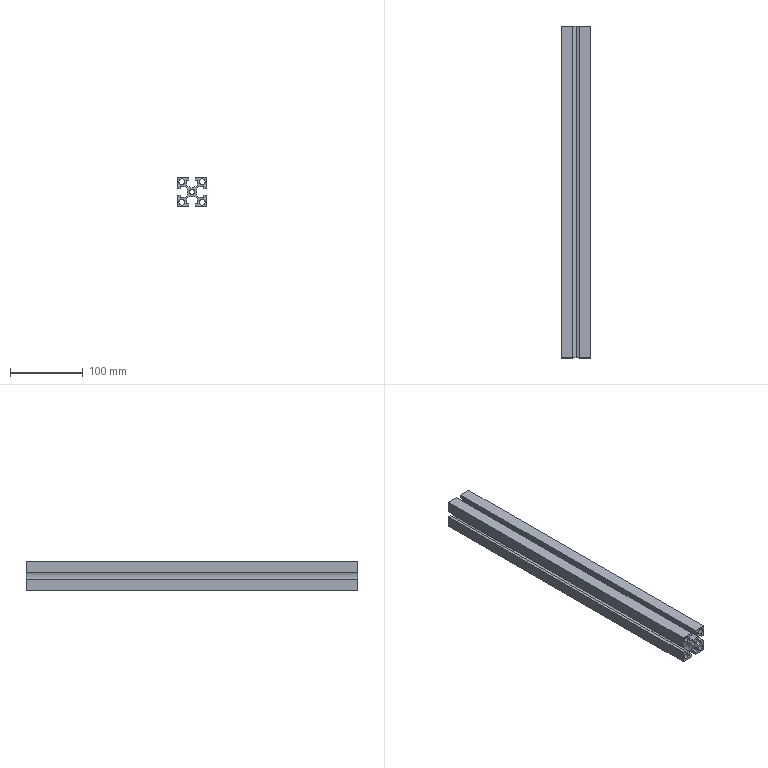Part | SolidWorks | features WeldMemberFeat 1, WeldmentFeature 1 | 1 solid | 49 faces | box 40 x 455 x 40 mm | volume 322038 mm3 | plane 34 | cylinder 15 | commonest cylinder face diameters 8 x8 19 x5 6.8 x2
STEP:
#1=CARTESIAN_POINT('',(14.,455.,-18.));
#2=VERTEX_POINT('',#1);
#3=CARTESIAN_POINT('',(14.,455.,-10.));
#4=VERTEX_POINT('',#3);
#5=CARTESIAN_POINT('',(14.,455.,-14.));
#6=DIRECTION('',(0.,1.,0.));
#7=DIRECTION('',(0.,0.,1.));
#8=AXIS2_PLACEMENT_3D('',#5,#6,#7);
#9=CIRCLE('',#8,4.);
#10=EDGE_CURVE('',#2,#4,#9,.T.);
#11=ORIENTED_EDGE('',*,*,#10,.T.);
#12=CARTESIAN_POINT('',(14.,0.,-10.));
#13=VERTEX_POINT('',#12);
#14=CARTESIAN_POINT('',(14.,455.,-10.));
#15=DIRECTION('',(0.,-1.,0.));
#16=VECTOR('',#15,1000.);
#17=LINE('',#14,#16);
#18=EDGE_CURVE('',#4,#13,#17,.T.);
#19=ORIENTED_EDGE('',*,*,#18,.T.);
#20=CARTESIAN_POINT('',(14.,0.,-18.));
#21=VERTEX_POINT('',#20);
#22=CARTESIAN_POINT('',(14.,0.,-14.));
#23=DIRECTION('',(0.,1.,0.));
#24=DIRECTION('',(0.,0.,1.));
#25=AXIS2_PLACEMENT_3D('',#22,#23,#24);
#26=CIRCLE('',#25,4.);
#27=EDGE_CURVE('',#21,#13,#26,.T.);
#28=ORIENTED_EDGE('',*,*,#27,.F.);
#29=CARTESIAN_POINT('',(14.,455.,-18.));
#30=DIRECTION('',(0.,-1.,0.));
#31=VECTOR('',#30,1000.);
#32=LINE('',#29,#31);
#33=EDGE_CURVE('',#2,#21,#32,.T.);
#34=ORIENTED_EDGE('',*,*,#33,.F.);
#35=EDGE_LOOP('',(#11,#19,#28,#34));
#36=FACE_OUTER_BOUND('',#35,.T.);
#37=CARTESIAN_POINT('',(14.,455.,-14.));
#38=DIRECTION('',(0.,-1.,0.));
#39=DIRECTION('',(0.,0.,-1.));
#40=AXIS2_PLACEMENT_3D('',#37,#38,#39);
#41=CYLINDRICAL_SURFACE('',#40,4.);
#42=ADVANCED_FACE('',(#36),#41,.F.);
#43=CARTESIAN_POINT('',(0.,455.,-3.4));
#44=VERTEX_POINT('',#43);
#45=CARTESIAN_POINT('',(0.,455.,3.4));
#46=VERTEX_POINT('',#45);
#47=CARTESIAN_POINT('',(0.,455.,0.));
#48=DIRECTION('',(0.,1.,0.));
#49=DIRECTION('',(0.,0.,1.));
#50=AXIS2_PLACEMENT_3D('',#47,#48,#49);
#51=CIRCLE('',#50,3.4);
#52=EDGE_CURVE('',#44,#46,#51,.T.);
#53=ORIENTED_EDGE('',*,*,#52,.T.);
#54=CARTESIAN_POINT('',(0.,0.,3.4));
#55=VERTEX_POINT('',#54);
#56=CARTESIAN_POINT('',(0.,455.,3.4));
#57=DIRECTION('',(0.,-1.,0.));
#58=VECTOR('',#57,1000.);
#59=LINE('',#56,#58);
#60=EDGE_CURVE('',#46,#55,#59,.T.);
#61=ORIENTED_EDGE('',*,*,#60,.T.);
#62=CARTESIAN_POINT('',(0.,0.,-3.4));
#63=VERTEX_POINT('',#62);
#64=CARTESIAN_POINT('',(0.,0.,0.));
#65=DIRECTION('',(0.,1.,0.));
#66=DIRECTION('',(0.,0.,1.));
#67=AXIS2_PLACEMENT_3D('',#64,#65,#66);
#68=CIRCLE('',#67,3.4);
#69=EDGE_CURVE('',#63,#55,#68,.T.);
#70=ORIENTED_EDGE('',*,*,#69,.F.);
#71=CARTESIAN_POINT('',(0.,455.,-3.4));
#72=DIRECTION('',(0.,-1.,0.));
#73=VECTOR('',#72,1000.);
#74=LINE('',#71,#73);
#75=EDGE_CURVE('',#44,#63,#74,.T.);
#76=ORIENTED_EDGE('',*,*,#75,.F.);
#77=EDGE_LOOP('',(#53,#61,#70,#76));
#78=FACE_OUTER_BOUND('',#77,.T.);
#79=CARTESIAN_POINT('',(0.,455.,0.));
#80=DIRECTION('',(0.,-1.,0.));
#81=DIRECTION('',(0.,0.,-1.));
#82=AXIS2_PLACEMENT_3D('',#79,#80,#81);
#83=CYLINDRICAL_SURFACE('',#82,3.4);
#84=ADVANCED_FACE('',(#78),#83,.F.);
#85=CARTESIAN_POINT('',(-14.,455.,-18.));
#86=VERTEX_POINT('',#85);
#87=CARTESIAN_POINT('',(-14.,455.,-10.));
#88=VERTEX_POINT('',#87);
#89=CARTESIAN_POINT('',(-14.,455.,-14.));
#90=DIRECTION('',(0.,1.,0.));
#91=DIRECTION('',(0.,0.,1.));
#92=AXIS2_PLACEMENT_3D('',#89,#90,#91);
#93=CIRCLE('',#92,4.);
#94=EDGE_CURVE('',#86,#88,#93,.T.);
#95=ORIENTED_EDGE('',*,*,#94,.T.);
#96=CARTESIAN_POINT('',(-14.,0.,-10.));
#97=VERTEX_POINT('',#96);
#98=CARTESIAN_POINT('',(-14.,455.,-10.));
#99=DIRECTION('',(0.,-1.,0.));
#100=VECTOR('',#99,1000.);
#101=LINE('',#98,#100);
#102=EDGE_CURVE('',#88,#97,#101,.T.);
#103=ORIENTED_EDGE('',*,*,#102,.T.);
#104=CARTESIAN_POINT('',(-14.,0.,-18.));
#105=VERTEX_POINT('',#104);
#106=CARTESIAN_POINT('',(-14.,0.,-14.));
#107=DIRECTION('',(0.,1.,0.));
#108=DIRECTION('',(0.,0.,1.));
#109=AXIS2_PLACEMENT_3D('',#106,#107,#108);
#110=CIRCLE('',#109,4.);
#111=EDGE_CURVE('',#105,#97,#110,.T.);
#112=ORIENTED_EDGE('',*,*,#111,.F.);
#113=CARTESIAN_POINT('',(-14.,455.,-18.));
#114=DIRECTION('',(0.,-1.,0.));
#115=VECTOR('',#114,1000.);
#116=LINE('',#113,#115);
#117=EDGE_CURVE('',#86,#105,#116,.T.);
#118=ORIENTED_EDGE('',*,*,#117,.F.);
#119=EDGE_LOOP('',(#95,#103,#112,#118));
#120=FACE_OUTER_BOUND('',#119,.T.);
#121=CARTESIAN_POINT('',(-14.,455.,-14.));
#122=DIRECTION('',(0.,-1.,0.));
#123=DIRECTION('',(0.,0.,-1.));
#124=AXIS2_PLACEMENT_3D('',#121,#122,#123);
#125=CYLINDRICAL_SURFACE('',#124,4.);
#126=ADVANCED_FACE('',(#120),#125,.F.);
#127=CARTESIAN_POINT('',(14.,455.,10.));
#128=VERTEX_POINT('',#127);
#129=CARTESIAN_POINT('',(14.,455.,18.));
#130=VERTEX_POINT('',#129);
#131=CARTESIAN_POINT('',(14.,455.,14.));
#132=DIRECTION('',(0.,1.,0.));
#133=DIRECTION('',(0.,0.,1.));
#134=AXIS2_PLACEMENT_3D('',#131,#132,#133);
#135=CIRCLE('',#134,4.);
#136=EDGE_CURVE('',#128,#130,#135,.T.);
#137=ORIENTED_EDGE('',*,*,#136,.T.);
#138=CARTESIAN_POINT('',(14.,0.,18.));
#139=VERTEX_POINT('',#138);
#140=CARTESIAN_POINT('',(14.,455.,18.));
#141=DIRECTION('',(0.,-1.,0.));
#142=VECTOR('',#141,1000.);
#143=LINE('',#140,#142);
#144=EDGE_CURVE('',#130,#139,#143,.T.);
#145=ORIENTED_EDGE('',*,*,#144,.T.);
#146=CARTESIAN_POINT('',(14.,0.,10.));
#147=VERTEX_POINT('',#146);
#148=CARTESIAN_POINT('',(14.,0.,14.));
#149=DIRECTION('',(0.,1.,0.));
#150=DIRECTION('',(0.,0.,1.));
#151=AXIS2_PLACEMENT_3D('',#148,#149,#150);
#152=CIRCLE('',#151,4.);
#153=EDGE_CURVE('',#147,#139,#152,.T.);
#154=ORIENTED_EDGE('',*,*,#153,.F.);
#155=CARTESIAN_POINT('',(14.,455.,10.));
#156=DIRECTION('',(0.,-1.,0.));
#157=VECTOR('',#156,1000.);
#158=LINE('',#155,#157);
#159=EDGE_CURVE('',#128,#147,#158,.T.);
#160=ORIENTED_EDGE('',*,*,#159,.F.);
#161=EDGE_LOOP('',(#137,#145,#154,#160));
#162=FACE_OUTER_BOUND('',#161,.T.);
#163=CARTESIAN_POINT('',(14.,455.,14.));
#164=DIRECTION('',(0.,-1.,0.));
#165=DIRECTION('',(0.,0.,-1.));
#166=AXIS2_PLACEMENT_3D('',#163,#164,#165);
#167=CYLINDRICAL_SURFACE('',#166,4.);
#168=ADVANCED_FACE('',(#162),#167,.F.);
#169=CARTESIAN_POINT('',(-14.,455.,10.));
#170=VERTEX_POINT('',#169);
#171=CARTESIAN_POINT('',(-14.,455.,18.));
#172=VERTEX_POINT('',#171);
#173=CARTESIAN_POINT('',(-14.,455.,14.));
#174=DIRECTION('',(0.,1.,0.));
#175=DIRECTION('',(0.,0.,1.));
#176=AXIS2_PLACEMENT_3D('',#173,#174,#175);
#177=CIRCLE('',#176,4.);
#178=EDGE_CURVE('',#170,#172,#177,.T.);
#179=ORIENTED_EDGE('',*,*,#178,.T.);
#180=CARTESIAN_POINT('',(-14.,0.,18.));
#181=VERTEX_POINT('',#180);
#182=CARTESIAN_POINT('',(-14.,455.,18.));
#183=DIRECTION('',(0.,-1.,0.));
#184=VECTOR('',#183,1000.);
#185=LINE('',#182,#184);
#186=EDGE_CURVE('',#172,#181,#185,.T.);
#187=ORIENTED_EDGE('',*,*,#186,.T.);
#188=CARTESIAN_POINT('',(-14.,0.,10.));
#189=VERTEX_POINT('',#188);
#190=CARTESIAN_POINT('',(-14.,0.,14.));
#191=DIRECTION('',(0.,1.,0.));
#192=DIRECTION('',(0.,0.,1.));
#193=AXIS2_PLACEMENT_3D('',#190,#191,#192);
#194=CIRCLE('',#193,4.);
#195=EDGE_CURVE('',#189,#181,#194,.T.);
#196=ORIENTED_EDGE('',*,*,#195,.F.);
#197=CARTESIAN_POINT('',(-14.,455.,10.));
#198=DIRECTION('',(0.,-1.,0.));
#199=VECTOR('',#198,1000.);
#200=LINE('',#197,#199);
#201=EDGE_CURVE('',#170,#189,#200,.T.);
#202=ORIENTED_EDGE('',*,*,#201,.F.);
#203=EDGE_LOOP('',(#179,#187,#196,#202));
#204=FACE_OUTER_BOUND('',#203,.T.);
#205=CARTESIAN_POINT('',(-14.,455.,14.));
#206=DIRECTION('',(0.,-1.,0.));
#207=DIRECTION('',(0.,0.,-1.));
#208=AXIS2_PLACEMENT_3D('',#205,#206,#207);
#209=CYLINDRICAL_SURFACE('',#208,4.);
#210=ADVANCED_FACE('',(#204),#209,.F.);
#211=CARTESIAN_POINT('',(0.,455.,6.));
#212=VERTEX_POINT('',#211);
#213=CARTESIAN_POINT('',(7.25,455.,9.361));
#214=VERTEX_POINT('',#213);
#215=CARTESIAN_POINT('',(0.,455.,15.5));
#216=DIRECTION('',(0.,-1.,0.));
#217=DIRECTION('',(0.,0.,1.));
#218=AXIS2_PLACEMENT_3D('',#215,#216,#217);
#219=CIRCLE('',#218,9.5);
#220=EDGE_CURVE('',#212,#214,#219,.T.);
#221=ORIENTED_EDGE('',*,*,#220,.F.);
#222=CARTESIAN_POINT('',(0.,0.,6.));
#223=VERTEX_POINT('',#222);
#224=CARTESIAN_POINT('',(0.,455.,6.));
#225=DIRECTION('',(0.,-1.,0.));
#226=VECTOR('',#225,1000.);
#227=LINE('',#224,#226);
#228=EDGE_CURVE('',#212,#223,#227,.T.);
#229=ORIENTED_EDGE('',*,*,#228,.T.);
#230=CARTESIAN_POINT('',(7.25,0.,9.361));
#231=VERTEX_POINT('',#230);
#232=CARTESIAN_POINT('',(0.,0.,15.5));
#233=DIRECTION('',(0.,-1.,0.));
#234=DIRECTION('',(0.,0.,1.));
#235=AXIS2_PLACEMENT_3D('',#232,#233,#234);
#236=CIRCLE('',#235,9.5);
#237=EDGE_CURVE('',#223,#231,#236,.T.);
#238=ORIENTED_EDGE('',*,*,#237,.T.);
#239=CARTESIAN_POINT('',(7.25,455.,9.361));
#240=DIRECTION('',(0.,-1.,0.));
#241=VECTOR('',#240,1000.);
#242=LINE('',#239,#241);
#243=EDGE_CURVE('',#214,#231,#242,.T.);
#244=ORIENTED_EDGE('',*,*,#243,.F.);
#245=EDGE_LOOP('',(#221,#229,#238,#244));
#246=FACE_OUTER_BOUND('',#245,.T.);
#247=CARTESIAN_POINT('',(0.,455.,15.5));
#248=DIRECTION('',(0.,-1.,0.));
#249=DIRECTION('',(0.,0.,-1.));
#250=AXIS2_PLACEMENT_3D('',#247,#248,#249);
#251=CYLINDRICAL_SURFACE('',#250,9.5);
#252=ADVANCED_FACE('',(#246),#251,.F.);
#253=CARTESIAN_POINT('',(-9.361,0.,-7.25));
#254=VERTEX_POINT('',#253);
#255=CARTESIAN_POINT('',(-9.361,0.,7.25));
#256=VERTEX_POINT('',#255);
#257=CARTESIAN_POINT('',(-15.5,0.,0.));
#258=DIRECTION('',(0.,-1.,0.));
#259=DIRECTION('',(0.,0.,1.));
#260=AXIS2_PLACEMENT_3D('',#257,#258,#259);
#261=CIRCLE('',#260,9.5);
#262=EDGE_CURVE('',#254,#256,#261,.T.);
#263=ORIENTED_EDGE('',*,*,#262,.T.);
#264=CARTESIAN_POINT('',(-9.361,455.,7.25));
#265=VERTEX_POINT('',#264);
#266=CARTESIAN_POINT('',(-9.361,455.,7.25));
#267=DIRECTION('',(0.,-1.,0.));
#268=VECTOR('',#267,1000.);
#269=LINE('',#266,#268);
#270=EDGE_CURVE('',#265,#256,#269,.T.);
#271=ORIENTED_EDGE('',*,*,#270,.F.);
#272=CARTESIAN_POINT('',(-9.361,455.,-7.25));
#273=VERTEX_POINT('',#272);
#274=CARTESIAN_POINT('',(-15.5,455.,0.));
#275=DIRECTION('',(0.,-1.,0.));
#276=DIRECTION('',(0.,0.,1.));
#277=AXIS2_PLACEMENT_3D('',#274,#275,#276);
#278=CIRCLE('',#277,9.5);
#279=EDGE_CURVE('',#273,#265,#278,.T.);
#280=ORIENTED_EDGE('',*,*,#279,.F.);
#281=CARTESIAN_POINT('',(-9.361,455.,-7.25));
#282=DIRECTION('',(0.,-1.,0.));
#283=VECTOR('',#282,1000.);
#284=LINE('',#281,#283);
#285=EDGE_CURVE('',#273,#254,#284,.T.);
#286=ORIENTED_EDGE('',*,*,#285,.T.);
#287=EDGE_LOOP('',(#263,#271,#280,#286));
#288=FACE_OUTER_BOUND('',#287,.T.);
#289=CARTESIAN_POINT('',(-15.5,455.,0.));
#290=DIRECTION('',(0.,-1.,0.));
#291=DIRECTION('',(0.,0.,-1.));
#292=AXIS2_PLACEMENT_3D('',#289,#290,#291);
#293=CYLINDRICAL_SURFACE('',#292,9.5);
#294=ADVANCED_FACE('',(#288),#293,.F.);
#295=CARTESIAN_POINT('',(-16.,0.,7.25));
#296=VERTEX_POINT('',#295);
#297=CARTESIAN_POINT('',(-9.361,0.,7.25));
#298=DIRECTION('',(-1.,0.,0.));
#299=VECTOR('',#298,1000.);
#300=LINE('',#297,#299);
#301=EDGE_CURVE('',#256,#296,#300,.T.);
#302=ORIENTED_EDGE('',*,*,#301,.T.);
#303=CARTESIAN_POINT('',(-16.,455.,7.25));
#304=VERTEX_POINT('',#303);
#305=CARTESIAN_POINT('',(-16.,455.,7.25));
#306=DIRECTION('',(0.,-1.,0.));
#307=VECTOR('',#306,1000.);
#308=LINE('',#305,#307);
#309=EDGE_CURVE('',#304,#296,#308,.T.);
#310=ORIENTED_EDGE('',*,*,#309,.F.);
#311=CARTESIAN_POINT('',(-9.361,455.,7.25));
#312=DIRECTION('',(-1.,0.,0.));
#313=VECTOR('',#312,1000.);
#314=LINE('',#311,#313);
#315=EDGE_CURVE('',#265,#304,#314,.T.);
#316=ORIENTED_EDGE('',*,*,#315,.F.);
#317=ORIENTED_EDGE('',*,*,#270,.T.);
#318=EDGE_LOOP('',(#302,#310,#316,#317));
#319=FACE_OUTER_BOUND('',#318,.T.);
#320=CARTESIAN_POINT('',(-9.361,455.,7.25));
#321=DIRECTION('',(0.,0.,1.));
#322=DIRECTION('',(1.,0.,0.));
#323=AXIS2_PLACEMENT_3D('',#320,#321,#322);
#324=PLANE('',#323);
#325=ADVANCED_FACE('',(#319),#324,.F.);
#326=CARTESIAN_POINT('',(-16.,0.,4.2));
#327=VERTEX_POINT('',#326);
#328=CARTESIAN_POINT('',(-16.,0.,7.25));
#329=DIRECTION('',(0.,0.,-1.));
#330=VECTOR('',#329,1000.);
#331=LINE('',#328,#330);
#332=EDGE_CURVE('',#296,#327,#331,.T.);
#333=ORIENTED_EDGE('',*,*,#332,.T.);
#334=CARTESIAN_POINT('',(-16.,455.,4.2));
#335=VERTEX_POINT('',#334);
#336=CARTESIAN_POINT('',(-16.,455.,4.2));
#337=DIRECTION('',(0.,-1.,0.));
#338=VECTOR('',#337,1000.);
#339=LINE('',#336,#338);
#340=EDGE_CURVE('',#335,#327,#339,.T.);
#341=ORIENTED_EDGE('',*,*,#340,.F.);
#342=CARTESIAN_POINT('',(-16.,455.,7.25));
#343=DIRECTION('',(0.,0.,-1.));
#344=VECTOR('',#343,1000.);
#345=LINE('',#342,#344);
#346=EDGE_CURVE('',#304,#335,#345,.T.);
#347=ORIENTED_EDGE('',*,*,#346,.F.);
#348=ORIENTED_EDGE('',*,*,#309,.T.);
#349=EDGE_LOOP('',(#333,#341,#347,#348));
#350=FACE_OUTER_BOUND('',#349,.T.);
#351=CARTESIAN_POINT('',(-16.,455.,7.25));
#352=DIRECTION('',(-1.,0.,0.));
#353=DIRECTION('',(0.,0.,1.));
#354=AXIS2_PLACEMENT_3D('',#351,#352,#353);
#355=PLANE('',#354);
#356=ADVANCED_FACE('',(#350),#355,.F.);
#357=CARTESIAN_POINT('',(-20.,0.,4.2));
#358=VERTEX_POINT('',#357);
#359=CARTESIAN_POINT('',(-16.,0.,4.2));
#360=DIRECTION('',(-1.,0.,0.));
#361=VECTOR('',#360,1000.);
#362=LINE('',#359,#361);
#363=EDGE_CURVE('',#327,#358,#362,.T.);
#364=ORIENTED_EDGE('',*,*,#363,.T.);
#365=CARTESIAN_POINT('',(-20.,455.,4.2));
#366=VERTEX_POINT('',#365);
#367=CARTESIAN_POINT('',(-20.,455.,4.2));
#368=DIRECTION('',(0.,-1.,0.));
#369=VECTOR('',#368,1000.);
#370=LINE('',#367,#369);
#371=EDGE_CURVE('',#366,#358,#370,.T.);
#372=ORIENTED_EDGE('',*,*,#371,.F.);
#373=CARTESIAN_POINT('',(-16.,455.,4.2));
#374=DIRECTION('',(-1.,0.,0.));
#375=VECTOR('',#374,1000.);
#376=LINE('',#373,#375);
#377=EDGE_CURVE('',#335,#366,#376,.T.);
#378=ORIENTED_EDGE('',*,*,#377,.F.);
#379=ORIENTED_EDGE('',*,*,#340,.T.);
#380=EDGE_LOOP('',(#364,#372,#378,#379));
#381=FACE_OUTER_BOUND('',#380,.T.);
#382=CARTESIAN_POINT('',(-16.,455.,4.2));
#383=DIRECTION('',(0.,0.,1.));
#384=DIRECTION('',(1.,0.,0.));
#385=AXIS2_PLACEMENT_3D('',#382,#383,#384);
#386=PLANE('',#385);
#387=ADVANCED_FACE('',(#381),#386,.F.);
#388=CARTESIAN_POINT('',(-20.,0.,20.));
#389=VERTEX_POINT('',#388);
#390=CARTESIAN_POINT('',(-20.,0.,4.2));
#391=DIRECTION('',(0.,0.,1.));
#392=VECTOR('',#391,1000.);
#393=LINE('',#390,#392);
#394=EDGE_CURVE('',#358,#389,#393,.T.);
#395=ORIENTED_EDGE('',*,*,#394,.T.);
#396=CARTESIAN_POINT('',(-20.,455.,20.));
#397=VERTEX_POINT('',#396);
#398=CARTESIAN_POINT('',(-20.,455.,20.));
#399=DIRECTION('',(0.,-1.,0.));
#400=VECTOR('',#399,1000.);
#401=LINE('',#398,#400);
#402=EDGE_CURVE('',#397,#389,#401,.T.);
#403=ORIENTED_EDGE('',*,*,#402,.F.);
#404=CARTESIAN_POINT('',(-20.,455.,4.2));
#405=DIRECTION('',(0.,0.,1.));
#406=VECTOR('',#405,1000.);
#407=LINE('',#404,#406);
#408=EDGE_CURVE('',#366,#397,#407,.T.);
#409=ORIENTED_EDGE('',*,*,#408,.F.);
#410=ORIENTED_EDGE('',*,*,#371,.T.);
#411=EDGE_LOOP('',(#395,#403,#409,#410));
#412=FACE_OUTER_BOUND('',#411,.T.);
#413=CARTESIAN_POINT('',(-20.,455.,4.2));
#414=DIRECTION('',(1.,0.,0.));
#415=DIRECTION('',(0.,0.,-1.));
#416=AXIS2_PLACEMENT_3D('',#413,#414,#415);
#417=PLANE('',#416);
#418=ADVANCED_FACE('',(#412),#417,.F.);
#419=CARTESIAN_POINT('',(-4.2,0.,20.));
#420=VERTEX_POINT('',#419);
#421=CARTESIAN_POINT('',(-20.,0.,20.));
#422=DIRECTION('',(1.,0.,0.));
#423=VECTOR('',#422,1000.);
#424=LINE('',#421,#423);
#425=EDGE_CURVE('',#389,#420,#424,.T.);
#426=ORIENTED_EDGE('',*,*,#425,.T.);
#427=CARTESIAN_POINT('',(-4.2,455.,20.));
#428=VERTEX_POINT('',#427);
#429=CARTESIAN_POINT('',(-4.2,455.,20.));
#430=DIRECTION('',(0.,-1.,0.));
#431=VECTOR('',#430,1000.);
#432=LINE('',#429,#431);
#433=EDGE_CURVE('',#428,#420,#432,.T.);
#434=ORIENTED_EDGE('',*,*,#433,.F.);
#435=CARTESIAN_POINT('',(-20.,455.,20.));
#436=DIRECTION('',(1.,0.,0.));
#437=VECTOR('',#436,1000.);
#438=LINE('',#435,#437);
#439=EDGE_CURVE('',#397,#428,#438,.T.);
#440=ORIENTED_EDGE('',*,*,#439,.F.);
#441=ORIENTED_EDGE('',*,*,#402,.T.);
#442=EDGE_LOOP('',(#426,#434,#440,#441));
#443=FACE_OUTER_BOUND('',#442,.T.);
#444=CARTESIAN_POINT('',(-20.,455.,20.));
#445=DIRECTION('',(0.,0.,-1.));
#446=DIRECTION('',(-1.,0.,0.));
#447=AXIS2_PLACEMENT_3D('',#444,#445,#446);
#448=PLANE('',#447);
#449=ADVANCED_FACE('',(#443),#448,.F.);
#450=CARTESIAN_POINT('',(-4.2,0.,16.));
#451=VERTEX_POINT('',#450);
#452=CARTESIAN_POINT('',(-4.2,0.,20.));
#453=DIRECTION('',(0.,0.,-1.));
#454=VECTOR('',#453,1000.);
#455=LINE('',#452,#454);
#456=EDGE_CURVE('',#420,#451,#455,.T.);
#457=ORIENTED_EDGE('',*,*,#456,.T.);
#458=CARTESIAN_POINT('',(-4.2,455.,16.));
#459=VERTEX_POINT('',#458);
#460=CARTESIAN_POINT('',(-4.2,455.,16.));
#461=DIRECTION('',(0.,-1.,0.));
#462=VECTOR('',#461,1000.);
#463=LINE('',#460,#462);
#464=EDGE_CURVE('',#459,#451,#463,.T.);
#465=ORIENTED_EDGE('',*,*,#464,.F.);
#466=CARTESIAN_POINT('',(-4.2,455.,20.));
#467=DIRECTION('',(0.,0.,-1.));
#468=VECTOR('',#467,1000.);
#469=LINE('',#466,#468);
#470=EDGE_CURVE('',#428,#459,#469,.T.);
#471=ORIENTED_EDGE('',*,*,#470,.F.);
#472=ORIENTED_EDGE('',*,*,#433,.T.);
#473=EDGE_LOOP('',(#457,#465,#471,#472));
#474=FACE_OUTER_BOUND('',#473,.T.);
#475=CARTESIAN_POINT('',(-4.2,455.,20.));
#476=DIRECTION('',(-1.,0.,0.));
#477=DIRECTION('',(0.,0.,1.));
#478=AXIS2_PLACEMENT_3D('',#475,#476,#477);
#479=PLANE('',#478);
#480=ADVANCED_FACE('',(#474),#479,.F.);
#481=CARTESIAN_POINT('',(-7.25,0.,16.));
#482=VERTEX_POINT('',#481);
#483=CARTESIAN_POINT('',(-4.2,0.,16.));
#484=DIRECTION('',(-1.,0.,0.));
#485=VECTOR('',#484,1000.);
#486=LINE('',#483,#485);
#487=EDGE_CURVE('',#451,#482,#486,.T.);
#488=ORIENTED_EDGE('',*,*,#487,.T.);
#489=CARTESIAN_POINT('',(-7.25,455.,16.));
#490=VERTEX_POINT('',#489);
#491=CARTESIAN_POINT('',(-7.25,455.,16.));
#492=DIRECTION('',(0.,-1.,0.));
#493=VECTOR('',#492,1000.);
#494=LINE('',#491,#493);
#495=EDGE_CURVE('',#490,#482,#494,.T.);
#496=ORIENTED_EDGE('',*,*,#495,.F.);
#497=CARTESIAN_POINT('',(-4.2,455.,16.));
#498=DIRECTION('',(-1.,0.,0.));
#499=VECTOR('',#498,1000.);
#500=LINE('',#497,#499);
#501=EDGE_CURVE('',#459,#490,#500,.T.);
#502=ORIENTED_EDGE('',*,*,#501,.F.);
#503=ORIENTED_EDGE('',*,*,#464,.T.);
#504=EDGE_LOOP('',(#488,#496,#502,#503));
#505=FACE_OUTER_BOUND('',#504,.T.);
#506=CARTESIAN_POINT('',(-4.2,455.,16.));
#507=DIRECTION('',(0.,0.,1.));
#508=DIRECTION('',(1.,0.,0.));
#509=AXIS2_PLACEMENT_3D('',#506,#507,#508);
#510=PLANE('',#509);
#511=ADVANCED_FACE('',(#505),#510,.F.);
#512=CARTESIAN_POINT('',(-7.25,0.,9.361));
#513=VERTEX_POINT('',#512);
#514=CARTESIAN_POINT('',(-7.25,0.,16.));
#515=DIRECTION('',(0.,0.,-1.));
#516=VECTOR('',#515,1000.);
#517=LINE('',#514,#516);
#518=EDGE_CURVE('',#482,#513,#517,.T.);
#519=ORIENTED_EDGE('',*,*,#518,.T.);
#520=CARTESIAN_POINT('',(-7.25,455.,9.361));
#521=VERTEX_POINT('',#520);
#522=CARTESIAN_POINT('',(-7.25,455.,9.361));
#523=DIRECTION('',(0.,-1.,0.));
#524=VECTOR('',#523,1000.);
#525=LINE('',#522,#524);
#526=EDGE_CURVE('',#521,#513,#525,.T.);
#527=ORIENTED_EDGE('',*,*,#526,.F.);
#528=CARTESIAN_POINT('',(-7.25,455.,16.));
#529=DIRECTION('',(0.,0.,-1.));
#530=VECTOR('',#529,1000.);
#531=LINE('',#528,#530);
#532=EDGE_CURVE('',#490,#521,#531,.T.);
#533=ORIENTED_EDGE('',*,*,#532,.F.);
#534=ORIENTED_EDGE('',*,*,#495,.T.);
#535=EDGE_LOOP('',(#519,#527,#533,#534));
#536=FACE_OUTER_BOUND('',#535,.T.);
#537=CARTESIAN_POINT('',(-7.25,455.,16.));
#538=DIRECTION('',(-1.,0.,0.));
#539=DIRECTION('',(0.,0.,1.));
#540=AXIS2_PLACEMENT_3D('',#537,#538,#539);
#541=PLANE('',#540);
#542=ADVANCED_FACE('',(#536),#541,.F.);
#543=ORIENTED_EDGE('',*,*,#228,.F.);
#544=CARTESIAN_POINT('',(0.,455.,15.5));
#545=DIRECTION('',(0.,-1.,0.));
#546=DIRECTION('',(0.,0.,1.));
#547=AXIS2_PLACEMENT_3D('',#544,#545,#546);
#548=CIRCLE('',#547,9.5);
#549=EDGE_CURVE('',#521,#212,#548,.T.);
#550=ORIENTED_EDGE('',*,*,#549,.F.);
#551=ORIENTED_EDGE('',*,*,#526,.T.);
#552=CARTESIAN_POINT('',(0.,0.,15.5));
#553=DIRECTION('',(0.,-1.,0.));
#554=DIRECTION('',(0.,0.,1.));
#555=AXIS2_PLACEMENT_3D('',#552,#553,#554);
#556=CIRCLE('',#555,9.5);
#557=EDGE_CURVE('',#513,#223,#556,.T.);
#558=ORIENTED_EDGE('',*,*,#557,.T.);
#559=EDGE_LOOP('',(#543,#550,#551,#558));
#560=FACE_OUTER_BOUND('',#559,.T.);
#561=CARTESIAN_POINT('',(0.,455.,15.5));
#562=DIRECTION('',(0.,-1.,0.));
#563=DIRECTION('',(0.,0.,-1.));
#564=AXIS2_PLACEMENT_3D('',#561,#562,#563);
#565=CYLINDRICAL_SURFACE('',#564,9.5);
#566=ADVANCED_FACE('',(#560),#565,.F.);
#567=CARTESIAN_POINT('',(7.25,0.,16.));
#568=VERTEX_POINT('',#567);
#569=CARTESIAN_POINT('',(7.25,0.,9.361));
#570=DIRECTION('',(0.,0.,1.));
#571=VECTOR('',#570,1000.);
#572=LINE('',#569,#571);
#573=EDGE_CURVE('',#231,#568,#572,.T.);
#574=ORIENTED_EDGE('',*,*,#573,.T.);
#575=CARTESIAN_POINT('',(7.25,455.,16.));
#576=VERTEX_POINT('',#575);
#577=CARTESIAN_POINT('',(7.25,455.,16.));
#578=DIRECTION('',(0.,-1.,0.));
#579=VECTOR('',#578,1000.);
#580=LINE('',#577,#579);
#581=EDGE_CURVE('',#576,#568,#580,.T.);
#582=ORIENTED_EDGE('',*,*,#581,.F.);
#583=CARTESIAN_POINT('',(7.25,455.,9.361));
#584=DIRECTION('',(0.,0.,1.));
#585=VECTOR('',#584,1000.);
#586=LINE('',#583,#585);
#587=EDGE_CURVE('',#214,#576,#586,.T.);
#588=ORIENTED_EDGE('',*,*,#587,.F.);
#589=ORIENTED_EDGE('',*,*,#243,.T.);
#590=EDGE_LOOP('',(#574,#582,#588,#589));
#591=FACE_OUTER_BOUND('',#590,.T.);
#592=CARTESIAN_POINT('',(7.25,455.,9.361));
#593=DIRECTION('',(1.,0.,0.));
#594=DIRECTION('',(0.,0.,-1.));
#595=AXIS2_PLACEMENT_3D('',#592,#593,#594);
#596=PLANE('',#595);
#597=ADVANCED_FACE('',(#591),#596,.F.);
#598=CARTESIAN_POINT('',(4.2,0.,16.));
#599=VERTEX_POINT('',#598);
#600=CARTESIAN_POINT('',(7.25,0.,16.));
#601=DIRECTION('',(-1.,0.,0.));
#602=VECTOR('',#601,1000.);
#603=LINE('',#600,#602);
#604=EDGE_CURVE('',#568,#599,#603,.T.);
#605=ORIENTED_EDGE('',*,*,#604,.T.);
#606=CARTESIAN_POINT('',(4.2,455.,16.));
#607=VERTEX_POINT('',#606);
#608=CARTESIAN_POINT('',(4.2,455.,16.));
#609=DIRECTION('',(0.,-1.,0.));
#610=VECTOR('',#609,1000.);
#611=LINE('',#608,#610);
#612=EDGE_CURVE('',#607,#599,#611,.T.);
#613=ORIENTED_EDGE('',*,*,#612,.F.);
#614=CARTESIAN_POINT('',(7.25,455.,16.));
#615=DIRECTION('',(-1.,0.,0.));
#616=VECTOR('',#615,1000.);
#617=LINE('',#614,#616);
#618=EDGE_CURVE('',#576,#607,#617,.T.);
#619=ORIENTED_EDGE('',*,*,#618,.F.);
#620=ORIENTED_EDGE('',*,*,#581,.T.);
#621=EDGE_LOOP('',(#605,#613,#619,#620));
#622=FACE_OUTER_BOUND('',#621,.T.);
#623=CARTESIAN_POINT('',(7.25,455.,16.));
#624=DIRECTION('',(0.,0.,1.));
#625=DIRECTION('',(1.,0.,0.));
#626=AXIS2_PLACEMENT_3D('',#623,#624,#625);
#627=PLANE('',#626);
#628=ADVANCED_FACE('',(#622),#627,.F.);
#629=CARTESIAN_POINT('',(4.2,0.,20.));
#630=VERTEX_POINT('',#629);
#631=CARTESIAN_POINT('',(4.2,0.,16.));
#632=DIRECTION('',(0.,0.,1.));
#633=VECTOR('',#632,1000.);
#634=LINE('',#631,#633);
#635=EDGE_CURVE('',#599,#630,#634,.T.);
#636=ORIENTED_EDGE('',*,*,#635,.T.);
#637=CARTESIAN_POINT('',(4.2,455.,20.));
#638=VERTEX_POINT('',#637);
#639=CARTESIAN_POINT('',(4.2,455.,20.));
#640=DIRECTION('',(0.,-1.,0.));
#641=VECTOR('',#640,1000.);
#642=LINE('',#639,#641);
#643=EDGE_CURVE('',#638,#630,#642,.T.);
#644=ORIENTED_EDGE('',*,*,#643,.F.);
#645=CARTESIAN_POINT('',(4.2,455.,16.));
#646=DIRECTION('',(0.,0.,1.));
#647=VECTOR('',#646,1000.);
#648=LINE('',#645,#647);
#649=EDGE_CURVE('',#607,#638,#648,.T.);
#650=ORIENTED_EDGE('',*,*,#649,.F.);
#651=ORIENTED_EDGE('',*,*,#612,.T.);
#652=EDGE_LOOP('',(#636,#644,#650,#651));
#653=FACE_OUTER_BOUND('',#652,.T.);
#654=CARTESIAN_POINT('',(4.2,455.,16.));
#655=DIRECTION('',(1.,0.,0.));
#656=DIRECTION('',(0.,0.,-1.));
#657=AXIS2_PLACEMENT_3D('',#654,#655,#656);
#658=PLANE('',#657);
#659=ADVANCED_FACE('',(#653),#658,.F.);
#660=CARTESIAN_POINT('',(20.,0.,20.));
#661=VERTEX_POINT('',#660);
#662=CARTESIAN_POINT('',(4.2,0.,20.));
#663=DIRECTION('',(1.,0.,0.));
#664=VECTOR('',#663,1000.);
#665=LINE('',#662,#664);
#666=EDGE_CURVE('',#630,#661,#665,.T.);
#667=ORIENTED_EDGE('',*,*,#666,.T.);
#668=CARTESIAN_POINT('',(20.,455.,20.));
#669=VERTEX_POINT('',#668);
#670=CARTESIAN_POINT('',(20.,455.,20.));
#671=DIRECTION('',(0.,-1.,0.));
#672=VECTOR('',#671,1000.);
#673=LINE('',#670,#672);
#674=EDGE_CURVE('',#669,#661,#673,.T.);
#675=ORIENTED_EDGE('',*,*,#674,.F.);
#676=CARTESIAN_POINT('',(4.2,455.,20.));
#677=DIRECTION('',(1.,0.,0.));
#678=VECTOR('',#677,1000.);
#679=LINE('',#676,#678);
#680=EDGE_CURVE('',#638,#669,#679,.T.);
#681=ORIENTED_EDGE('',*,*,#680,.F.);
#682=ORIENTED_EDGE('',*,*,#643,.T.);
#683=EDGE_LOOP('',(#667,#675,#681,#682));
#684=FACE_OUTER_BOUND('',#683,.T.);
#685=CARTESIAN_POINT('',(4.2,455.,20.));
#686=DIRECTION('',(0.,0.,-1.));
#687=DIRECTION('',(-1.,0.,0.));
#688=AXIS2_PLACEMENT_3D('',#685,#686,#687);
#689=PLANE('',#688);
#690=ADVANCED_FACE('',(#684),#689,.F.);
#691=CARTESIAN_POINT('',(20.,0.,4.2));
#692=VERTEX_POINT('',#691);
#693=CARTESIAN_POINT('',(20.,0.,20.));
#694=DIRECTION('',(0.,0.,-1.));
#695=VECTOR('',#694,1000.);
#696=LINE('',#693,#695);
#697=EDGE_CURVE('',#661,#692,#696,.T.);
#698=ORIENTED_EDGE('',*,*,#697,.T.);
#699=CARTESIAN_POINT('',(20.,455.,4.2));
#700=VERTEX_POINT('',#699);
#701=CARTESIAN_POINT('',(20.,455.,4.2));
#702=DIRECTION('',(0.,-1.,0.));
#703=VECTOR('',#702,1000.);
#704=LINE('',#701,#703);
#705=EDGE_CURVE('',#700,#692,#704,.T.);
#706=ORIENTED_EDGE('',*,*,#705,.F.);
#707=CARTESIAN_POINT('',(20.,455.,20.));
#708=DIRECTION('',(0.,0.,-1.));
#709=VECTOR('',#708,1000.);
#710=LINE('',#707,#709);
#711=EDGE_CURVE('',#669,#700,#710,.T.);
#712=ORIENTED_EDGE('',*,*,#711,.F.);
#713=ORIENTED_EDGE('',*,*,#674,.T.);
#714=EDGE_LOOP('',(#698,#706,#712,#713));
#715=FACE_OUTER_BOUND('',#714,.T.);
#716=CARTESIAN_POINT('',(20.,455.,20.));
#717=DIRECTION('',(-1.,0.,0.));
#718=DIRECTION('',(0.,0.,1.));
#719=AXIS2_PLACEMENT_3D('',#716,#717,#718);
#720=PLANE('',#719);
#721=ADVANCED_FACE('',(#715),#720,.F.);
#722=CARTESIAN_POINT('',(16.,0.,4.2));
#723=VERTEX_POINT('',#722);
#724=CARTESIAN_POINT('',(20.,0.,4.2));
#725=DIRECTION('',(-1.,0.,0.));
#726=VECTOR('',#725,1000.);
#727=LINE('',#724,#726);
#728=EDGE_CURVE('',#692,#723,#727,.T.);
#729=ORIENTED_EDGE('',*,*,#728,.T.);
#730=CARTESIAN_POINT('',(16.,455.,4.2));
#731=VERTEX_POINT('',#730);
#732=CARTESIAN_POINT('',(16.,455.,4.2));
#733=DIRECTION('',(0.,-1.,0.));
#734=VECTOR('',#733,1000.);
#735=LINE('',#732,#734);
#736=EDGE_CURVE('',#731,#723,#735,.T.);
#737=ORIENTED_EDGE('',*,*,#736,.F.);
#738=CARTESIAN_POINT('',(20.,455.,4.2));
#739=DIRECTION('',(-1.,0.,0.));
#740=VECTOR('',#739,1000.);
#741=LINE('',#738,#740);
#742=EDGE_CURVE('',#700,#731,#741,.T.);
#743=ORIENTED_EDGE('',*,*,#742,.F.);
#744=ORIENTED_EDGE('',*,*,#705,.T.);
#745=EDGE_LOOP('',(#729,#737,#743,#744));
#746=FACE_OUTER_BOUND('',#745,.T.);
#747=CARTESIAN_POINT('',(20.,455.,4.2));
#748=DIRECTION('',(0.,0.,1.));
#749=DIRECTION('',(1.,0.,0.));
#750=AXIS2_PLACEMENT_3D('',#747,#748,#749);
#751=PLANE('',#750);
#752=ADVANCED_FACE('',(#746),#751,.F.);
#753=CARTESIAN_POINT('',(16.,0.,7.25));
#754=VERTEX_POINT('',#753);
#755=CARTESIAN_POINT('',(16.,0.,4.2));
#756=DIRECTION('',(0.,0.,1.));
#757=VECTOR('',#756,1000.);
#758=LINE('',#755,#757);
#759=EDGE_CURVE('',#723,#754,#758,.T.);
#760=ORIENTED_EDGE('',*,*,#759,.T.);
#761=CARTESIAN_POINT('',(16.,455.,7.25));
#762=VERTEX_POINT('',#761);
#763=CARTESIAN_POINT('',(16.,455.,7.25));
#764=DIRECTION('',(0.,-1.,0.));
#765=VECTOR('',#764,1000.);
#766=LINE('',#763,#765);
#767=EDGE_CURVE('',#762,#754,#766,.T.);
#768=ORIENTED_EDGE('',*,*,#767,.F.);
#769=CARTESIAN_POINT('',(16.,455.,4.2));
#770=DIRECTION('',(0.,0.,1.));
#771=VECTOR('',#770,1000.);
#772=LINE('',#769,#771);
#773=EDGE_CURVE('',#731,#762,#772,.T.);
#774=ORIENTED_EDGE('',*,*,#773,.F.);
#775=ORIENTED_EDGE('',*,*,#736,.T.);
#776=EDGE_LOOP('',(#760,#768,#774,#775));
#777=FACE_OUTER_BOUND('',#776,.T.);
#778=CARTESIAN_POINT('',(16.,455.,4.2));
#779=DIRECTION('',(1.,0.,0.));
#780=DIRECTION('',(0.,0.,-1.));
#781=AXIS2_PLACEMENT_3D('',#778,#779,#780);
#782=PLANE('',#781);
#783=ADVANCED_FACE('',(#777),#782,.F.);
#784=CARTESIAN_POINT('',(9.361,0.,7.25));
#785=VERTEX_POINT('',#784);
#786=CARTESIAN_POINT('',(16.,0.,7.25));
#787=DIRECTION('',(-1.,0.,0.));
#788=VECTOR('',#787,1000.);
#789=LINE('',#786,#788);
#790=EDGE_CURVE('',#754,#785,#789,.T.);
#791=ORIENTED_EDGE('',*,*,#790,.T.);
#792=CARTESIAN_POINT('',(9.361,455.,7.25));
#793=VERTEX_POINT('',#792);
#794=CARTESIAN_POINT('',(9.361,455.,7.25));
#795=DIRECTION('',(0.,-1.,0.));
#796=VECTOR('',#795,1000.);
#797=LINE('',#794,#796);
#798=EDGE_CURVE('',#793,#785,#797,.T.);
#799=ORIENTED_EDGE('',*,*,#798,.F.);
#800=CARTESIAN_POINT('',(16.,455.,7.25));
#801=DIRECTION('',(-1.,0.,0.));
#802=VECTOR('',#801,1000.);
#803=LINE('',#800,#802);
#804=EDGE_CURVE('',#762,#793,#803,.T.);
#805=ORIENTED_EDGE('',*,*,#804,.F.);
#806=ORIENTED_EDGE('',*,*,#767,.T.);
#807=EDGE_LOOP('',(#791,#799,#805,#806));
#808=FACE_OUTER_BOUND('',#807,.T.);
#809=CARTESIAN_POINT('',(16.,455.,7.25));
#810=DIRECTION('',(0.,0.,1.));
#811=DIRECTION('',(1.,0.,0.));
#812=AXIS2_PLACEMENT_3D('',#809,#810,#811);
#813=PLANE('',#812);
#814=ADVANCED_FACE('',(#808),#813,.F.);
#815=CARTESIAN_POINT('',(9.361,0.,-7.25));
#816=VERTEX_POINT('',#815);
#817=CARTESIAN_POINT('',(15.5,0.,0.));
#818=DIRECTION('',(0.,-1.,0.));
#819=DIRECTION('',(0.,0.,1.));
#820=AXIS2_PLACEMENT_3D('',#817,#818,#819);
#821=CIRCLE('',#820,9.5);
#822=EDGE_CURVE('',#785,#816,#821,.T.);
#823=ORIENTED_EDGE('',*,*,#822,.T.);
#824=CARTESIAN_POINT('',(9.361,455.,-7.25));
#825=VERTEX_POINT('',#824);
#826=CARTESIAN_POINT('',(9.361,455.,-7.25));
#827=DIRECTION('',(0.,-1.,0.));
#828=VECTOR('',#827,1000.);
#829=LINE('',#826,#828);
#830=EDGE_CURVE('',#825,#816,#829,.T.);
#831=ORIENTED_EDGE('',*,*,#830,.F.);
#832=CARTESIAN_POINT('',(15.5,455.,0.));
#833=DIRECTION('',(0.,-1.,0.));
#834=DIRECTION('',(0.,0.,1.));
#835=AXIS2_PLACEMENT_3D('',#832,#833,#834);
#836=CIRCLE('',#835,9.5);
#837=EDGE_CURVE('',#793,#825,#836,.T.);
#838=ORIENTED_EDGE('',*,*,#837,.F.);
#839=ORIENTED_EDGE('',*,*,#798,.T.);
#840=EDGE_LOOP('',(#823,#831,#838,#839));
#841=FACE_OUTER_BOUND('',#840,.T.);
#842=CARTESIAN_POINT('',(15.5,455.,0.));
#843=DIRECTION('',(0.,-1.,0.));
#844=DIRECTION('',(0.,0.,-1.));
#845=AXIS2_PLACEMENT_3D('',#842,#843,#844);
#846=CYLINDRICAL_SURFACE('',#845,9.5);
#847=ADVANCED_FACE('',(#841),#846,.F.);
#848=CARTESIAN_POINT('',(16.,0.,-7.25));
#849=VERTEX_POINT('',#848);
#850=CARTESIAN_POINT('',(9.361,0.,-7.25));
#851=DIRECTION('',(1.,0.,0.));
#852=VECTOR('',#851,1000.);
#853=LINE('',#850,#852);
#854=EDGE_CURVE('',#816,#849,#853,.T.);
#855=ORIENTED_EDGE('',*,*,#854,.T.);
#856=CARTESIAN_POINT('',(16.,455.,-7.25));
#857=VERTEX_POINT('',#856);
#858=CARTESIAN_POINT('',(16.,455.,-7.25));
#859=DIRECTION('',(0.,-1.,0.));
#860=VECTOR('',#859,1000.);
#861=LINE('',#858,#860);
#862=EDGE_CURVE('',#857,#849,#861,.T.);
#863=ORIENTED_EDGE('',*,*,#862,.F.);
#864=CARTESIAN_POINT('',(9.361,455.,-7.25));
#865=DIRECTION('',(1.,0.,0.));
#866=VECTOR('',#865,1000.);
#867=LINE('',#864,#866);
#868=EDGE_CURVE('',#825,#857,#867,.T.);
#869=ORIENTED_EDGE('',*,*,#868,.F.);
#870=ORIENTED_EDGE('',*,*,#830,.T.);
#871=EDGE_LOOP('',(#855,#863,#869,#870));
#872=FACE_OUTER_BOUND('',#871,.T.);
#873=CARTESIAN_POINT('',(9.361,455.,-7.25));
#874=DIRECTION('',(0.,0.,-1.));
#875=DIRECTION('',(-1.,0.,0.));
#876=AXIS2_PLACEMENT_3D('',#873,#874,#875);
#877=PLANE('',#876);
#878=ADVANCED_FACE('',(#872),#877,.F.);
#879=CARTESIAN_POINT('',(16.,0.,-4.2));
#880=VERTEX_POINT('',#879);
#881=CARTESIAN_POINT('',(16.,0.,-7.25));
#882=DIRECTION('',(0.,0.,1.));
#883=VECTOR('',#882,1000.);
#884=LINE('',#881,#883);
#885=EDGE_CURVE('',#849,#880,#884,.T.);
#886=ORIENTED_EDGE('',*,*,#885,.T.);
#887=CARTESIAN_POINT('',(16.,455.,-4.2));
#888=VERTEX_POINT('',#887);
#889=CARTESIAN_POINT('',(16.,455.,-4.2));
#890=DIRECTION('',(0.,-1.,0.));
#891=VECTOR('',#890,1000.);
#892=LINE('',#889,#891);
#893=EDGE_CURVE('',#888,#880,#892,.T.);
#894=ORIENTED_EDGE('',*,*,#893,.F.);
#895=CARTESIAN_POINT('',(16.,455.,-7.25));
#896=DIRECTION('',(0.,0.,1.));
#897=VECTOR('',#896,1000.);
#898=LINE('',#895,#897);
#899=EDGE_CURVE('',#857,#888,#898,.T.);
#900=ORIENTED_EDGE('',*,*,#899,.F.);
#901=ORIENTED_EDGE('',*,*,#862,.T.);
#902=EDGE_LOOP('',(#886,#894,#900,#901));
#903=FACE_OUTER_BOUND('',#902,.T.);
#904=CARTESIAN_POINT('',(16.,455.,-7.25));
#905=DIRECTION('',(1.,0.,0.));
#906=DIRECTION('',(0.,0.,-1.));
#907=AXIS2_PLACEMENT_3D('',#904,#905,#906);
#908=PLANE('',#907);
#909=ADVANCED_FACE('',(#903),#908,.F.);
#910=CARTESIAN_POINT('',(20.,0.,-4.2));
#911=VERTEX_POINT('',#910);
#912=CARTESIAN_POINT('',(16.,0.,-4.2));
#913=DIRECTION('',(1.,0.,0.));
#914=VECTOR('',#913,1000.);
#915=LINE('',#912,#914);
#916=EDGE_CURVE('',#880,#911,#915,.T.);
#917=ORIENTED_EDGE('',*,*,#916,.T.);
#918=CARTESIAN_POINT('',(20.,455.,-4.2));
#919=VERTEX_POINT('',#918);
#920=CARTESIAN_POINT('',(20.,455.,-4.2));
#921=DIRECTION('',(0.,-1.,0.));
#922=VECTOR('',#921,1000.);
#923=LINE('',#920,#922);
#924=EDGE_CURVE('',#919,#911,#923,.T.);
#925=ORIENTED_EDGE('',*,*,#924,.F.);
#926=CARTESIAN_POINT('',(16.,455.,-4.2));
#927=DIRECTION('',(1.,0.,0.));
#928=VECTOR('',#927,1000.);
#929=LINE('',#926,#928);
#930=EDGE_CURVE('',#888,#919,#929,.T.);
#931=ORIENTED_EDGE('',*,*,#930,.F.);
#932=ORIENTED_EDGE('',*,*,#893,.T.);
#933=EDGE_LOOP('',(#917,#925,#931,#932));
#934=FACE_OUTER_BOUND('',#933,.T.);
#935=CARTESIAN_POINT('',(16.,455.,-4.2));
#936=DIRECTION('',(0.,0.,-1.));
#937=DIRECTION('',(-1.,0.,0.));
#938=AXIS2_PLACEMENT_3D('',#935,#936,#937);
#939=PLANE('',#938);
#940=ADVANCED_FACE('',(#934),#939,.F.);
#941=CARTESIAN_POINT('',(20.,0.,-20.));
#942=VERTEX_POINT('',#941);
#943=CARTESIAN_POINT('',(20.,0.,-4.2));
#944=DIRECTION('',(0.,0.,-1.));
#945=VECTOR('',#944,1000.);
#946=LINE('',#943,#945);
#947=EDGE_CURVE('',#911,#942,#946,.T.);
#948=ORIENTED_EDGE('',*,*,#947,.T.);
#949=CARTESIAN_POINT('',(20.,455.,-20.));
#950=VERTEX_POINT('',#949);
#951=CARTESIAN_POINT('',(20.,455.,-20.));
#952=DIRECTION('',(0.,-1.,0.));
#953=VECTOR('',#952,1000.);
#954=LINE('',#951,#953);
#955=EDGE_CURVE('',#950,#942,#954,.T.);
#956=ORIENTED_EDGE('',*,*,#955,.F.);
#957=CARTESIAN_POINT('',(20.,455.,-4.2));
#958=DIRECTION('',(0.,0.,-1.));
#959=VECTOR('',#958,1000.);
#960=LINE('',#957,#959);
#961=EDGE_CURVE('',#919,#950,#960,.T.);
#962=ORIENTED_EDGE('',*,*,#961,.F.);
#963=ORIENTED_EDGE('',*,*,#924,.T.);
#964=EDGE_LOOP('',(#948,#956,#962,#963));
#965=FACE_OUTER_BOUND('',#964,.T.);
#966=CARTESIAN_POINT('',(20.,455.,-4.2));
#967=DIRECTION('',(-1.,0.,0.));
#968=DIRECTION('',(0.,0.,1.));
#969=AXIS2_PLACEMENT_3D('',#966,#967,#968);
#970=PLANE('',#969);
#971=ADVANCED_FACE('',(#965),#970,.F.);
#972=CARTESIAN_POINT('',(4.2,0.,-20.));
#973=VERTEX_POINT('',#972);
#974=CARTESIAN_POINT('',(20.,0.,-20.));
#975=DIRECTION('',(-1.,0.,0.));
#976=VECTOR('',#975,1000.);
#977=LINE('',#974,#976);
#978=EDGE_CURVE('',#942,#973,#977,.T.);
#979=ORIENTED_EDGE('',*,*,#978,.T.);
#980=CARTESIAN_POINT('',(4.2,455.,-20.));
#981=VERTEX_POINT('',#980);
#982=CARTESIAN_POINT('',(4.2,455.,-20.));
#983=DIRECTION('',(0.,-1.,0.));
#984=VECTOR('',#983,1000.);
#985=LINE('',#982,#984);
#986=EDGE_CURVE('',#981,#973,#985,.T.);
#987=ORIENTED_EDGE('',*,*,#986,.F.);
#988=CARTESIAN_POINT('',(20.,455.,-20.));
#989=DIRECTION('',(-1.,0.,0.));
#990=VECTOR('',#989,1000.);
#991=LINE('',#988,#990);
#992=EDGE_CURVE('',#950,#981,#991,.T.);
#993=ORIENTED_EDGE('',*,*,#992,.F.);
#994=ORIENTED_EDGE('',*,*,#955,.T.);
#995=EDGE_LOOP('',(#979,#987,#993,#994));
#996=FACE_OUTER_BOUND('',#995,.T.);
#997=CARTESIAN_POINT('',(20.,455.,-20.));
#998=DIRECTION('',(0.,0.,1.));
#999=DIRECTION('',(1.,0.,0.));
#1000=AXIS2_PLACEMENT_3D('',#997,#998,#999);
#1001=PLANE('',#1000);
#1002=ADVANCED_FACE('',(#996),#1001,.F.);
#1003=CARTESIAN_POINT('',(4.2,0.,-16.));
#1004=VERTEX_POINT('',#1003);
#1005=CARTESIAN_POINT('',(4.2,0.,-20.));
#1006=DIRECTION('',(0.,0.,1.));
#1007=VECTOR('',#1006,1000.);
#1008=LINE('',#1005,#1007);
#1009=EDGE_CURVE('',#973,#1004,#1008,.T.);
#1010=ORIENTED_EDGE('',*,*,#1009,.T.);
#1011=CARTESIAN_POINT('',(4.2,455.,-16.));
#1012=VERTEX_POINT('',#1011);
#1013=CARTESIAN_POINT('',(4.2,455.,-16.));
#1014=DIRECTION('',(0.,-1.,0.));
#1015=VECTOR('',#1014,1000.);
#1016=LINE('',#1013,#1015);
#1017=EDGE_CURVE('',#1012,#1004,#1016,.T.);
#1018=ORIENTED_EDGE('',*,*,#1017,.F.);
#1019=CARTESIAN_POINT('',(4.2,455.,-20.));
#1020=DIRECTION('',(0.,0.,1.));
#1021=VECTOR('',#1020,1000.);
#1022=LINE('',#1019,#1021);
#1023=EDGE_CURVE('',#981,#1012,#1022,.T.);
#1024=ORIENTED_EDGE('',*,*,#1023,.F.);
#1025=ORIENTED_EDGE('',*,*,#986,.T.);
#1026=EDGE_LOOP('',(#1010,#1018,#1024,#1025));
#1027=FACE_OUTER_BOUND('',#1026,.T.);
#1028=CARTESIAN_POINT('',(4.2,455.,-20.));
#1029=DIRECTION('',(1.,0.,0.));
#1030=DIRECTION('',(0.,0.,-1.));
#1031=AXIS2_PLACEMENT_3D('',#1028,#1029,#1030);
#1032=PLANE('',#1031);
#1033=ADVANCED_FACE('',(#1027),#1032,.F.);
#1034=CARTESIAN_POINT('',(7.25,0.,-16.));
#1035=VERTEX_POINT('',#1034);
#1036=CARTESIAN_POINT('',(4.2,0.,-16.));
#1037=DIRECTION('',(1.,0.,0.));
#1038=VECTOR('',#1037,1000.);
#1039=LINE('',#1036,#1038);
#1040=EDGE_CURVE('',#1004,#1035,#1039,.T.);
#1041=ORIENTED_EDGE('',*,*,#1040,.T.);
#1042=CARTESIAN_POINT('',(7.25,455.,-16.));
#1043=VERTEX_POINT('',#1042);
#1044=CARTESIAN_POINT('',(7.25,455.,-16.));
#1045=DIRECTION('',(0.,-1.,0.));
#1046=VECTOR('',#1045,1000.);
#1047=LINE('',#1044,#1046);
#1048=EDGE_CURVE('',#1043,#1035,#1047,.T.);
#1049=ORIENTED_EDGE('',*,*,#1048,.F.);
#1050=CARTESIAN_POINT('',(4.2,455.,-16.));
#1051=DIRECTION('',(1.,0.,0.));
#1052=VECTOR('',#1051,1000.);
#1053=LINE('',#1050,#1052);
#1054=EDGE_CURVE('',#1012,#1043,#1053,.T.);
#1055=ORIENTED_EDGE('',*,*,#1054,.F.);
#1056=ORIENTED_EDGE('',*,*,#1017,.T.);
#1057=EDGE_LOOP('',(#1041,#1049,#1055,#1056));
#1058=FACE_OUTER_BOUND('',#1057,.T.);
#1059=CARTESIAN_POINT('',(4.2,455.,-16.));
#1060=DIRECTION('',(0.,0.,-1.));
#1061=DIRECTION('',(-1.,0.,0.));
#1062=AXIS2_PLACEMENT_3D('',#1059,#1060,#1061);
#1063=PLANE('',#1062);
#1064=ADVANCED_FACE('',(#1058),#1063,.F.);
#1065=CARTESIAN_POINT('',(7.25,0.,-9.361));
#1066=VERTEX_POINT('',#1065);
#1067=CARTESIAN_POINT('',(7.25,0.,-16.));
#1068=DIRECTION('',(0.,0.,1.));
#1069=VECTOR('',#1068,1000.);
#1070=LINE('',#1067,#1069);
#1071=EDGE_CURVE('',#1035,#1066,#1070,.T.);
#1072=ORIENTED_EDGE('',*,*,#1071,.T.);
#1073=CARTESIAN_POINT('',(7.25,455.,-9.361));
#1074=VERTEX_POINT('',#1073);
#1075=CARTESIAN_POINT('',(7.25,455.,-9.361));
#1076=DIRECTION('',(0.,-1.,0.));
#1077=VECTOR('',#1076,1000.);
#1078=LINE('',#1075,#1077);
#1079=EDGE_CURVE('',#1074,#1066,#1078,.T.);
#1080=ORIENTED_EDGE('',*,*,#1079,.F.);
#1081=CARTESIAN_POINT('',(7.25,455.,-16.));
#1082=DIRECTION('',(0.,0.,1.));
#1083=VECTOR('',#1082,1000.);
#1084=LINE('',#1081,#1083);
#1085=EDGE_CURVE('',#1043,#1074,#1084,.T.);
#1086=ORIENTED_EDGE('',*,*,#1085,.F.);
#1087=ORIENTED_EDGE('',*,*,#1048,.T.);
#1088=EDGE_LOOP('',(#1072,#1080,#1086,#1087));
#1089=FACE_OUTER_BOUND('',#1088,.T.);
#1090=CARTESIAN_POINT('',(7.25,455.,-16.));
#1091=DIRECTION('',(1.,0.,0.));
#1092=DIRECTION('',(0.,0.,-1.));
#1093=AXIS2_PLACEMENT_3D('',#1090,#1091,#1092);
#1094=PLANE('',#1093);
#1095=ADVANCED_FACE('',(#1089),#1094,.F.);
#1096=CARTESIAN_POINT('',(-7.25,0.,-9.361));
#1097=VERTEX_POINT('',#1096);
#1098=CARTESIAN_POINT('',(0.,0.,-15.5));
#1099=DIRECTION('',(0.,-1.,0.));
#1100=DIRECTION('',(0.,0.,1.));
#1101=AXIS2_PLACEMENT_3D('',#1098,#1099,#1100);
#1102=CIRCLE('',#1101,9.5);
#1103=EDGE_CURVE('',#1066,#1097,#1102,.T.);
#1104=ORIENTED_EDGE('',*,*,#1103,.T.);
#1105=CARTESIAN_POINT('',(-7.25,455.,-9.361));
#1106=VERTEX_POINT('',#1105);
#1107=CARTESIAN_POINT('',(-7.25,455.,-9.361));
#1108=DIRECTION('',(0.,-1.,0.));
#1109=VECTOR('',#1108,1000.);
#1110=LINE('',#1107,#1109);
#1111=EDGE_CURVE('',#1106,#1097,#1110,.T.);
#1112=ORIENTED_EDGE('',*,*,#1111,.F.);
#1113=CARTESIAN_POINT('',(0.,455.,-15.5));
#1114=DIRECTION('',(0.,-1.,0.));
#1115=DIRECTION('',(0.,0.,1.));
#1116=AXIS2_PLACEMENT_3D('',#1113,#1114,#1115);
#1117=CIRCLE('',#1116,9.5);
#1118=EDGE_CURVE('',#1074,#1106,#1117,.T.);
#1119=ORIENTED_EDGE('',*,*,#1118,.F.);
#1120=ORIENTED_EDGE('',*,*,#1079,.T.);
#1121=EDGE_LOOP('',(#1104,#1112,#1119,#1120));
#1122=FACE_OUTER_BOUND('',#1121,.T.);
#1123=CARTESIAN_POINT('',(0.,455.,-15.5));
#1124=DIRECTION('',(0.,-1.,0.));
#1125=DIRECTION('',(0.,0.,-1.));
#1126=AXIS2_PLACEMENT_3D('',#1123,#1124,#1125);
#1127=CYLINDRICAL_SURFACE('',#1126,9.5);
#1128=ADVANCED_FACE('',(#1122),#1127,.F.);
#1129=CARTESIAN_POINT('',(-7.25,0.,-16.));
#1130=VERTEX_POINT('',#1129);
#1131=CARTESIAN_POINT('',(-7.25,0.,-9.361));
#1132=DIRECTION('',(0.,0.,-1.));
#1133=VECTOR('',#1132,1000.);
#1134=LINE('',#1131,#1133);
#1135=EDGE_CURVE('',#1097,#1130,#1134,.T.);
#1136=ORIENTED_EDGE('',*,*,#1135,.T.);
#1137=CARTESIAN_POINT('',(-7.25,455.,-16.));
#1138=VERTEX_POINT('',#1137);
#1139=CARTESIAN_POINT('',(-7.25,455.,-16.));
#1140=DIRECTION('',(0.,-1.,0.));
#1141=VECTOR('',#1140,1000.);
#1142=LINE('',#1139,#1141);
#1143=EDGE_CURVE('',#1138,#1130,#1142,.T.);
#1144=ORIENTED_EDGE('',*,*,#1143,.F.);
#1145=CARTESIAN_POINT('',(-7.25,455.,-9.361));
#1146=DIRECTION('',(0.,0.,-1.));
#1147=VECTOR('',#1146,1000.);
#1148=LINE('',#1145,#1147);
#1149=EDGE_CURVE('',#1106,#1138,#1148,.T.);
#1150=ORIENTED_EDGE('',*,*,#1149,.F.);
#1151=ORIENTED_EDGE('',*,*,#1111,.T.);
#1152=EDGE_LOOP('',(#1136,#1144,#1150,#1151));
#1153=FACE_OUTER_BOUND('',#1152,.T.);
#1154=CARTESIAN_POINT('',(-7.25,455.,-9.361));
#1155=DIRECTION('',(-1.,0.,0.));
#1156=DIRECTION('',(0.,0.,1.));
#1157=AXIS2_PLACEMENT_3D('',#1154,#1155,#1156);
#1158=PLANE('',#1157);
#1159=ADVANCED_FACE('',(#1153),#1158,.F.);
#1160=CARTESIAN_POINT('',(-4.2,0.,-16.));
#1161=VERTEX_POINT('',#1160);
#1162=CARTESIAN_POINT('',(-7.25,0.,-16.));
#1163=DIRECTION('',(1.,0.,0.));
#1164=VECTOR('',#1163,1000.);
#1165=LINE('',#1162,#1164);
#1166=EDGE_CURVE('',#1130,#1161,#1165,.T.);
#1167=ORIENTED_EDGE('',*,*,#1166,.T.);
#1168=CARTESIAN_POINT('',(-4.2,455.,-16.));
#1169=VERTEX_POINT('',#1168);
#1170=CARTESIAN_POINT('',(-4.2,455.,-16.));
#1171=DIRECTION('',(0.,-1.,0.));
#1172=VECTOR('',#1171,1000.);
#1173=LINE('',#1170,#1172);
#1174=EDGE_CURVE('',#1169,#1161,#1173,.T.);
#1175=ORIENTED_EDGE('',*,*,#1174,.F.);
#1176=CARTESIAN_POINT('',(-7.25,455.,-16.));
#1177=DIRECTION('',(1.,0.,0.));
#1178=VECTOR('',#1177,1000.);
#1179=LINE('',#1176,#1178);
#1180=EDGE_CURVE('',#1138,#1169,#1179,.T.);
#1181=ORIENTED_EDGE('',*,*,#1180,.F.);
#1182=ORIENTED_EDGE('',*,*,#1143,.T.);
#1183=EDGE_LOOP('',(#1167,#1175,#1181,#1182));
#1184=FACE_OUTER_BOUND('',#1183,.T.);
#1185=CARTESIAN_POINT('',(-7.25,455.,-16.));
#1186=DIRECTION('',(0.,0.,-1.));
#1187=DIRECTION('',(-1.,0.,0.));
#1188=AXIS2_PLACEMENT_3D('',#1185,#1186,#1187);
#1189=PLANE('',#1188);
#1190=ADVANCED_FACE('',(#1184),#1189,.F.);
#1191=CARTESIAN_POINT('',(-4.2,0.,-20.));
#1192=VERTEX_POINT('',#1191);
#1193=CARTESIAN_POINT('',(-4.2,0.,-16.));
#1194=DIRECTION('',(0.,0.,-1.));
#1195=VECTOR('',#1194,1000.);
#1196=LINE('',#1193,#1195);
#1197=EDGE_CURVE('',#1161,#1192,#1196,.T.);
#1198=ORIENTED_EDGE('',*,*,#1197,.T.);
#1199=CARTESIAN_POINT('',(-4.2,455.,-20.));
#1200=VERTEX_POINT('',#1199);
#1201=CARTESIAN_POINT('',(-4.2,455.,-20.));
#1202=DIRECTION('',(0.,-1.,0.));
#1203=VECTOR('',#1202,1000.);
#1204=LINE('',#1201,#1203);
#1205=EDGE_CURVE('',#1200,#1192,#1204,.T.);
#1206=ORIENTED_EDGE('',*,*,#1205,.F.);
#1207=CARTESIAN_POINT('',(-4.2,455.,-16.));
#1208=DIRECTION('',(0.,0.,-1.));
#1209=VECTOR('',#1208,1000.);
#1210=LINE('',#1207,#1209);
#1211=EDGE_CURVE('',#1169,#1200,#1210,.T.);
#1212=ORIENTED_EDGE('',*,*,#1211,.F.);
#1213=ORIENTED_EDGE('',*,*,#1174,.T.);
#1214=EDGE_LOOP('',(#1198,#1206,#1212,#1213));
#1215=FACE_OUTER_BOUND('',#1214,.T.);
#1216=CARTESIAN_POINT('',(-4.2,455.,-16.));
#1217=DIRECTION('',(-1.,0.,0.));
#1218=DIRECTION('',(0.,0.,1.));
#1219=AXIS2_PLACEMENT_3D('',#1216,#1217,#1218);
#1220=PLANE('',#1219);
#1221=ADVANCED_FACE('',(#1215),#1220,.F.);
#1222=CARTESIAN_POINT('',(-20.,0.,-20.));
#1223=VERTEX_POINT('',#1222);
#1224=CARTESIAN_POINT('',(-4.2,0.,-20.));
#1225=DIRECTION('',(-1.,0.,0.));
#1226=VECTOR('',#1225,1000.);
#1227=LINE('',#1224,#1226);
#1228=EDGE_CURVE('',#1192,#1223,#1227,.T.);
#1229=ORIENTED_EDGE('',*,*,#1228,.T.);
#1230=CARTESIAN_POINT('',(-20.,455.,-20.));
#1231=VERTEX_POINT('',#1230);
#1232=CARTESIAN_POINT('',(-20.,455.,-20.));
#1233=DIRECTION('',(0.,-1.,0.));
#1234=VECTOR('',#1233,1000.);
#1235=LINE('',#1232,#1234);
#1236=EDGE_CURVE('',#1231,#1223,#1235,.T.);
#1237=ORIENTED_EDGE('',*,*,#1236,.F.);
#1238=CARTESIAN_POINT('',(-4.2,455.,-20.));
#1239=DIRECTION('',(-1.,0.,0.));
#1240=VECTOR('',#1239,1000.);
#1241=LINE('',#1238,#1240);
#1242=EDGE_CURVE('',#1200,#1231,#1241,.T.);
#1243=ORIENTED_EDGE('',*,*,#1242,.F.);
#1244=ORIENTED_EDGE('',*,*,#1205,.T.);
#1245=EDGE_LOOP('',(#1229,#1237,#1243,#1244));
#1246=FACE_OUTER_BOUND('',#1245,.T.);
#1247=CARTESIAN_POINT('',(-4.2,455.,-20.));
#1248=DIRECTION('',(0.,0.,1.));
#1249=DIRECTION('',(1.,0.,0.));
#1250=AXIS2_PLACEMENT_3D('',#1247,#1248,#1249);
#1251=PLANE('',#1250);
#1252=ADVANCED_FACE('',(#1246),#1251,.F.);
#1253=CARTESIAN_POINT('',(-20.,0.,-4.2));
#1254=VERTEX_POINT('',#1253);
#1255=CARTESIAN_POINT('',(-20.,0.,-20.));
#1256=DIRECTION('',(0.,0.,1.));
#1257=VECTOR('',#1256,1000.);
#1258=LINE('',#1255,#1257);
#1259=EDGE_CURVE('',#1223,#1254,#1258,.T.);
#1260=ORIENTED_EDGE('',*,*,#1259,.T.);
#1261=CARTESIAN_POINT('',(-20.,455.,-4.2));
#1262=VERTEX_POINT('',#1261);
#1263=CARTESIAN_POINT('',(-20.,455.,-4.2));
#1264=DIRECTION('',(0.,-1.,0.));
#1265=VECTOR('',#1264,1000.);
#1266=LINE('',#1263,#1265);
#1267=EDGE_CURVE('',#1262,#1254,#1266,.T.);
#1268=ORIENTED_EDGE('',*,*,#1267,.F.);
#1269=CARTESIAN_POINT('',(-20.,455.,-20.));
#1270=DIRECTION('',(0.,0.,1.));
#1271=VECTOR('',#1270,1000.);
#1272=LINE('',#1269,#1271);
#1273=EDGE_CURVE('',#1231,#1262,#1272,.T.);
#1274=ORIENTED_EDGE('',*,*,#1273,.F.);
#1275=ORIENTED_EDGE('',*,*,#1236,.T.);
#1276=EDGE_LOOP('',(#1260,#1268,#1274,#1275));
#1277=FACE_OUTER_BOUND('',#1276,.T.);
#1278=CARTESIAN_POINT('',(-20.,455.,-20.));
#1279=DIRECTION('',(1.,0.,0.));
#1280=DIRECTION('',(0.,0.,-1.));
#1281=AXIS2_PLACEMENT_3D('',#1278,#1279,#1280);
#1282=PLANE('',#1281);
#1283=ADVANCED_FACE('',(#1277),#1282,.F.);
#1284=CARTESIAN_POINT('',(-16.,0.,-4.2));
#1285=VERTEX_POINT('',#1284);
#1286=CARTESIAN_POINT('',(-20.,0.,-4.2));
#1287=DIRECTION('',(1.,0.,0.));
#1288=VECTOR('',#1287,1000.);
#1289=LINE('',#1286,#1288);
#1290=EDGE_CURVE('',#1254,#1285,#1289,.T.);
#1291=ORIENTED_EDGE('',*,*,#1290,.T.);
#1292=CARTESIAN_POINT('',(-16.,455.,-4.2));
#1293=VERTEX_POINT('',#1292);
#1294=CARTESIAN_POINT('',(-16.,455.,-4.2));
#1295=DIRECTION('',(0.,-1.,0.));
#1296=VECTOR('',#1295,1000.);
#1297=LINE('',#1294,#1296);
#1298=EDGE_CURVE('',#1293,#1285,#1297,.T.);
#1299=ORIENTED_EDGE('',*,*,#1298,.F.);
#1300=CARTESIAN_POINT('',(-20.,455.,-4.2));
#1301=DIRECTION('',(1.,0.,0.));
#1302=VECTOR('',#1301,1000.);
#1303=LINE('',#1300,#1302);
#1304=EDGE_CURVE('',#1262,#1293,#1303,.T.);
#1305=ORIENTED_EDGE('',*,*,#1304,.F.);
#1306=ORIENTED_EDGE('',*,*,#1267,.T.);
#1307=EDGE_LOOP('',(#1291,#1299,#1305,#1306));
#1308=FACE_OUTER_BOUND('',#1307,.T.);
#1309=CARTESIAN_POINT('',(-20.,455.,-4.2));
#1310=DIRECTION('',(0.,0.,-1.));
#1311=DIRECTION('',(-1.,0.,0.));
#1312=AXIS2_PLACEMENT_3D('',#1309,#1310,#1311);
#1313=PLANE('',#1312);
#1314=ADVANCED_FACE('',(#1308),#1313,.F.);
#1315=CARTESIAN_POINT('',(-16.,0.,-7.25));
#1316=VERTEX_POINT('',#1315);
#1317=CARTESIAN_POINT('',(-16.,0.,-4.2));
#1318=DIRECTION('',(0.,0.,-1.));
#1319=VECTOR('',#1318,1000.);
#1320=LINE('',#1317,#1319);
#1321=EDGE_CURVE('',#1285,#1316,#1320,.T.);
#1322=ORIENTED_EDGE('',*,*,#1321,.T.);
#1323=CARTESIAN_POINT('',(-16.,455.,-7.25));
#1324=VERTEX_POINT('',#1323);
#1325=CARTESIAN_POINT('',(-16.,455.,-7.25));
#1326=DIRECTION('',(0.,-1.,0.));
#1327=VECTOR('',#1326,1000.);
#1328=LINE('',#1325,#1327);
#1329=EDGE_CURVE('',#1324,#1316,#1328,.T.);
#1330=ORIENTED_EDGE('',*,*,#1329,.F.);
#1331=CARTESIAN_POINT('',(-16.,455.,-4.2));
#1332=DIRECTION('',(0.,0.,-1.));
#1333=VECTOR('',#1332,1000.);
#1334=LINE('',#1331,#1333);
#1335=EDGE_CURVE('',#1293,#1324,#1334,.T.);
#1336=ORIENTED_EDGE('',*,*,#1335,.F.);
#1337=ORIENTED_EDGE('',*,*,#1298,.T.);
#1338=EDGE_LOOP('',(#1322,#1330,#1336,#1337));
#1339=FACE_OUTER_BOUND('',#1338,.T.);
#1340=CARTESIAN_POINT('',(-16.,455.,-4.2));
#1341=DIRECTION('',(-1.,0.,0.));
#1342=DIRECTION('',(0.,0.,1.));
#1343=AXIS2_PLACEMENT_3D('',#1340,#1341,#1342);
#1344=PLANE('',#1343);
#1345=ADVANCED_FACE('',(#1339),#1344,.F.);
#1346=ORIENTED_EDGE('',*,*,#186,.F.);
#1347=CARTESIAN_POINT('',(-14.,455.,14.));
#1348=DIRECTION('',(0.,1.,0.));
#1349=DIRECTION('',(0.,0.,1.));
#1350=AXIS2_PLACEMENT_3D('',#1347,#1348,#1349);
#1351=CIRCLE('',#1350,4.);
#1352=EDGE_CURVE('',#172,#170,#1351,.T.);
#1353=ORIENTED_EDGE('',*,*,#1352,.T.);
#1354=ORIENTED_EDGE('',*,*,#201,.T.);
#1355=CARTESIAN_POINT('',(-14.,0.,14.));
#1356=DIRECTION('',(0.,1.,0.));
#1357=DIRECTION('',(0.,0.,1.));
#1358=AXIS2_PLACEMENT_3D('',#1355,#1356,#1357);
#1359=CIRCLE('',#1358,4.);
#1360=EDGE_CURVE('',#181,#189,#1359,.T.);
#1361=ORIENTED_EDGE('',*,*,#1360,.F.);
#1362=EDGE_LOOP('',(#1346,#1353,#1354,#1361));
#1363=FACE_OUTER_BOUND('',#1362,.T.);
#1364=CARTESIAN_POINT('',(-14.,455.,14.));
#1365=DIRECTION('',(0.,-1.,0.));
#1366=DIRECTION('',(0.,0.,-1.));
#1367=AXIS2_PLACEMENT_3D('',#1364,#1365,#1366);
#1368=CYLINDRICAL_SURFACE('',#1367,4.);
#1369=ADVANCED_FACE('',(#1363),#1368,.F.);
#1370=ORIENTED_EDGE('',*,*,#144,.F.);
#1371=CARTESIAN_POINT('',(14.,455.,14.));
#1372=DIRECTION('',(0.,1.,0.));
#1373=DIRECTION('',(0.,0.,1.));
#1374=AXIS2_PLACEMENT_3D('',#1371,#1372,#1373);
#1375=CIRCLE('',#1374,4.);
#1376=EDGE_CURVE('',#130,#128,#1375,.T.);
#1377=ORIENTED_EDGE('',*,*,#1376,.T.);
#1378=ORIENTED_EDGE('',*,*,#159,.T.);
#1379=CARTESIAN_POINT('',(14.,0.,14.));
#1380=DIRECTION('',(0.,1.,0.));
#1381=DIRECTION('',(0.,0.,1.));
#1382=AXIS2_PLACEMENT_3D('',#1379,#1380,#1381);
#1383=CIRCLE('',#1382,4.);
#1384=EDGE_CURVE('',#139,#147,#1383,.T.);
#1385=ORIENTED_EDGE('',*,*,#1384,.F.);
#1386=EDGE_LOOP('',(#1370,#1377,#1378,#1385));
#1387=FACE_OUTER_BOUND('',#1386,.T.);
#1388=CARTESIAN_POINT('',(14.,455.,14.));
#1389=DIRECTION('',(0.,-1.,0.));
#1390=DIRECTION('',(0.,0.,-1.));
#1391=AXIS2_PLACEMENT_3D('',#1388,#1389,#1390);
#1392=CYLINDRICAL_SURFACE('',#1391,4.);
#1393=ADVANCED_FACE('',(#1387),#1392,.F.);
#1394=ORIENTED_EDGE('',*,*,#102,.F.);
#1395=CARTESIAN_POINT('',(-14.,455.,-14.));
#1396=DIRECTION('',(0.,1.,0.));
#1397=DIRECTION('',(0.,0.,1.));
#1398=AXIS2_PLACEMENT_3D('',#1395,#1396,#1397);
#1399=CIRCLE('',#1398,4.);
#1400=EDGE_CURVE('',#88,#86,#1399,.T.);
#1401=ORIENTED_EDGE('',*,*,#1400,.T.);
#1402=ORIENTED_EDGE('',*,*,#117,.T.);
#1403=CARTESIAN_POINT('',(-14.,0.,-14.));
#1404=DIRECTION('',(0.,1.,0.));
#1405=DIRECTION('',(0.,0.,1.));
#1406=AXIS2_PLACEMENT_3D('',#1403,#1404,#1405);
#1407=CIRCLE('',#1406,4.);
#1408=EDGE_CURVE('',#97,#105,#1407,.T.);
#1409=ORIENTED_EDGE('',*,*,#1408,.F.);
#1410=EDGE_LOOP('',(#1394,#1401,#1402,#1409));
#1411=FACE_OUTER_BOUND('',#1410,.T.);
#1412=CARTESIAN_POINT('',(-14.,455.,-14.));
#1413=DIRECTION('',(0.,-1.,0.));
#1414=DIRECTION('',(0.,0.,-1.));
#1415=AXIS2_PLACEMENT_3D('',#1412,#1413,#1414);
#1416=CYLINDRICAL_SURFACE('',#1415,4.);
#1417=ADVANCED_FACE('',(#1411),#1416,.F.);
#1418=ORIENTED_EDGE('',*,*,#60,.F.);
#1419=CARTESIAN_POINT('',(0.,455.,0.));
#1420=DIRECTION('',(0.,1.,0.));
#1421=DIRECTION('',(0.,0.,1.));
#1422=AXIS2_PLACEMENT_3D('',#1419,#1420,#1421);
#1423=CIRCLE('',#1422,3.4);
#1424=EDGE_CURVE('',#46,#44,#1423,.T.);
#1425=ORIENTED_EDGE('',*,*,#1424,.T.);
#1426=ORIENTED_EDGE('',*,*,#75,.T.);
#1427=CARTESIAN_POINT('',(0.,0.,0.));
#1428=DIRECTION('',(0.,1.,0.));
#1429=DIRECTION('',(0.,0.,1.));
#1430=AXIS2_PLACEMENT_3D('',#1427,#1428,#1429);
#1431=CIRCLE('',#1430,3.4);
#1432=EDGE_CURVE('',#55,#63,#1431,.T.);
#1433=ORIENTED_EDGE('',*,*,#1432,.F.);
#1434=EDGE_LOOP('',(#1418,#1425,#1426,#1433));
#1435=FACE_OUTER_BOUND('',#1434,.T.);
#1436=CARTESIAN_POINT('',(0.,455.,0.));
#1437=DIRECTION('',(0.,-1.,0.));
#1438=DIRECTION('',(0.,0.,-1.));
#1439=AXIS2_PLACEMENT_3D('',#1436,#1437,#1438);
#1440=CYLINDRICAL_SURFACE('',#1439,3.4);
#1441=ADVANCED_FACE('',(#1435),#1440,.F.);
#1442=ORIENTED_EDGE('',*,*,#18,.F.);
#1443=CARTESIAN_POINT('',(14.,455.,-14.));
#1444=DIRECTION('',(0.,1.,0.));
#1445=DIRECTION('',(0.,0.,1.));
#1446=AXIS2_PLACEMENT_3D('',#1443,#1444,#1445);
#1447=CIRCLE('',#1446,4.);
#1448=EDGE_CURVE('',#4,#2,#1447,.T.);
#1449=ORIENTED_EDGE('',*,*,#1448,.T.);
#1450=ORIENTED_EDGE('',*,*,#33,.T.);
#1451=CARTESIAN_POINT('',(14.,0.,-14.));
#1452=DIRECTION('',(0.,1.,0.));
#1453=DIRECTION('',(0.,0.,1.));
#1454=AXIS2_PLACEMENT_3D('',#1451,#1452,#1453);
#1455=CIRCLE('',#1454,4.);
#1456=EDGE_CURVE('',#13,#21,#1455,.T.);
#1457=ORIENTED_EDGE('',*,*,#1456,.F.);
#1458=EDGE_LOOP('',(#1442,#1449,#1450,#1457));
#1459=FACE_OUTER_BOUND('',#1458,.T.);
#1460=CARTESIAN_POINT('',(14.,455.,-14.));
#1461=DIRECTION('',(0.,-1.,0.));
#1462=DIRECTION('',(0.,0.,-1.));
#1463=AXIS2_PLACEMENT_3D('',#1460,#1461,#1462);
#1464=CYLINDRICAL_SURFACE('',#1463,4.);
#1465=ADVANCED_FACE('',(#1459),#1464,.F.);
#1466=CARTESIAN_POINT('',(-16.,0.,-7.25));
#1467=DIRECTION('',(1.,0.,0.));
#1468=VECTOR('',#1467,1000.);
#1469=LINE('',#1466,#1468);
#1470=EDGE_CURVE('',#1316,#254,#1469,.T.);
#1471=ORIENTED_EDGE('',*,*,#1470,.T.);
#1472=ORIENTED_EDGE('',*,*,#285,.F.);
#1473=CARTESIAN_POINT('',(-16.,455.,-7.25));
#1474=DIRECTION('',(1.,0.,0.));
#1475=VECTOR('',#1474,1000.);
#1476=LINE('',#1473,#1475);
#1477=EDGE_CURVE('',#1324,#273,#1476,.T.);
#1478=ORIENTED_EDGE('',*,*,#1477,.F.);
#1479=ORIENTED_EDGE('',*,*,#1329,.T.);
#1480=EDGE_LOOP('',(#1471,#1472,#1478,#1479));
#1481=FACE_OUTER_BOUND('',#1480,.T.);
#1482=CARTESIAN_POINT('',(-16.,455.,-7.25));
#1483=DIRECTION('',(0.,0.,-1.));
#1484=DIRECTION('',(-1.,0.,0.));
#1485=AXIS2_PLACEMENT_3D('',#1482,#1483,#1484);
#1486=PLANE('',#1485);
#1487=ADVANCED_FACE('',(#1481),#1486,.F.);
#1488=ORIENTED_EDGE('',*,*,#10,.F.);
#1489=ORIENTED_EDGE('',*,*,#1448,.F.);
#1490=EDGE_LOOP('',(#1488,#1489));
#1491=FACE_BOUND('',#1490,.T.);
#1492=ORIENTED_EDGE('',*,*,#52,.F.);
#1493=ORIENTED_EDGE('',*,*,#1424,.F.);
#1494=EDGE_LOOP('',(#1492,#1493));
#1495=FACE_BOUND('',#1494,.T.);
#1496=ORIENTED_EDGE('',*,*,#94,.F.);
#1497=ORIENTED_EDGE('',*,*,#1400,.F.);
#1498=EDGE_LOOP('',(#1496,#1497));
#1499=FACE_BOUND('',#1498,.T.);
#1500=ORIENTED_EDGE('',*,*,#136,.F.);
#1501=ORIENTED_EDGE('',*,*,#1376,.F.);
#1502=EDGE_LOOP('',(#1500,#1501));
#1503=FACE_BOUND('',#1502,.T.);
#1504=ORIENTED_EDGE('',*,*,#178,.F.);
#1505=ORIENTED_EDGE('',*,*,#1352,.F.);
#1506=EDGE_LOOP('',(#1504,#1505));
#1507=FACE_BOUND('',#1506,.T.);
#1508=ORIENTED_EDGE('',*,*,#279,.T.);
#1509=ORIENTED_EDGE('',*,*,#315,.T.);
#1510=ORIENTED_EDGE('',*,*,#346,.T.);
#1511=ORIENTED_EDGE('',*,*,#377,.T.);
#1512=ORIENTED_EDGE('',*,*,#408,.T.);
#1513=ORIENTED_EDGE('',*,*,#439,.T.);
#1514=ORIENTED_EDGE('',*,*,#470,.T.);
#1515=ORIENTED_EDGE('',*,*,#501,.T.);
#1516=ORIENTED_EDGE('',*,*,#532,.T.);
#1517=ORIENTED_EDGE('',*,*,#549,.T.);
#1518=ORIENTED_EDGE('',*,*,#220,.T.);
#1519=ORIENTED_EDGE('',*,*,#587,.T.);
#1520=ORIENTED_EDGE('',*,*,#618,.T.);
#1521=ORIENTED_EDGE('',*,*,#649,.T.);
#1522=ORIENTED_EDGE('',*,*,#680,.T.);
#1523=ORIENTED_EDGE('',*,*,#711,.T.);
#1524=ORIENTED_EDGE('',*,*,#742,.T.);
#1525=ORIENTED_EDGE('',*,*,#773,.T.);
#1526=ORIENTED_EDGE('',*,*,#804,.T.);
#1527=ORIENTED_EDGE('',*,*,#837,.T.);
#1528=ORIENTED_EDGE('',*,*,#868,.T.);
#1529=ORIENTED_EDGE('',*,*,#899,.T.);
#1530=ORIENTED_EDGE('',*,*,#930,.T.);
#1531=ORIENTED_EDGE('',*,*,#961,.T.);
#1532=ORIENTED_EDGE('',*,*,#992,.T.);
#1533=ORIENTED_EDGE('',*,*,#1023,.T.);
#1534=ORIENTED_EDGE('',*,*,#1054,.T.);
#1535=ORIENTED_EDGE('',*,*,#1085,.T.);
#1536=ORIENTED_EDGE('',*,*,#1118,.T.);
#1537=ORIENTED_EDGE('',*,*,#1149,.T.);
#1538=ORIENTED_EDGE('',*,*,#1180,.T.);
#1539=ORIENTED_EDGE('',*,*,#1211,.T.);
#1540=ORIENTED_EDGE('',*,*,#1242,.T.);
#1541=ORIENTED_EDGE('',*,*,#1273,.T.);
#1542=ORIENTED_EDGE('',*,*,#1304,.T.);
#1543=ORIENTED_EDGE('',*,*,#1335,.T.);
#1544=ORIENTED_EDGE('',*,*,#1477,.T.);
#1545=EDGE_LOOP('',(#1508,#1509,#1510,#1511,#1512,#1513,#1514,#1515,#1516,#1517,#1518,#1519,#1520,#1521,#1522,#1523,#1524,#1525,#1526,#1527,#1528,#1529,#1530,#1531,#1532,#1533,#1534,#1535,#1536,#1537,#1538,#1539,#1540,#1541,#1542,#1543,#1544));
#1546=FACE_OUTER_BOUND('',#1545,.T.);
#1547=CARTESIAN_POINT('',(-15.5,455.,0.));
#1548=DIRECTION('',(0.,1.,0.));
#1549=DIRECTION('',(0.,0.,1.));
#1550=AXIS2_PLACEMENT_3D('',#1547,#1548,#1549);
#1551=PLANE('',#1550);
#1552=ADVANCED_FACE('',(#1491,#1495,#1499,#1503,#1507,#1546),#1551,.T.);
#1553=ORIENTED_EDGE('',*,*,#27,.T.);
#1554=ORIENTED_EDGE('',*,*,#1456,.T.);
#1555=EDGE_LOOP('',(#1553,#1554));
#1556=FACE_BOUND('',#1555,.T.);
#1557=ORIENTED_EDGE('',*,*,#69,.T.);
#1558=ORIENTED_EDGE('',*,*,#1432,.T.);
#1559=EDGE_LOOP('',(#1557,#1558));
#1560=FACE_BOUND('',#1559,.T.);
#1561=ORIENTED_EDGE('',*,*,#111,.T.);
#1562=ORIENTED_EDGE('',*,*,#1408,.T.);
#1563=EDGE_LOOP('',(#1561,#1562));
#1564=FACE_BOUND('',#1563,.T.);
#1565=ORIENTED_EDGE('',*,*,#153,.T.);
#1566=ORIENTED_EDGE('',*,*,#1384,.T.);
#1567=EDGE_LOOP('',(#1565,#1566));
#1568=FACE_BOUND('',#1567,.T.);
#1569=ORIENTED_EDGE('',*,*,#195,.T.);
#1570=ORIENTED_EDGE('',*,*,#1360,.T.);
#1571=EDGE_LOOP('',(#1569,#1570));
#1572=FACE_BOUND('',#1571,.T.);
#1573=ORIENTED_EDGE('',*,*,#262,.F.);
#1574=ORIENTED_EDGE('',*,*,#1470,.F.);
#1575=ORIENTED_EDGE('',*,*,#1321,.F.);
#1576=ORIENTED_EDGE('',*,*,#1290,.F.);
#1577=ORIENTED_EDGE('',*,*,#1259,.F.);
#1578=ORIENTED_EDGE('',*,*,#1228,.F.);
#1579=ORIENTED_EDGE('',*,*,#1197,.F.);
#1580=ORIENTED_EDGE('',*,*,#1166,.F.);
#1581=ORIENTED_EDGE('',*,*,#1135,.F.);
#1582=ORIENTED_EDGE('',*,*,#1103,.F.);
#1583=ORIENTED_EDGE('',*,*,#1071,.F.);
#1584=ORIENTED_EDGE('',*,*,#1040,.F.);
#1585=ORIENTED_EDGE('',*,*,#1009,.F.);
#1586=ORIENTED_EDGE('',*,*,#978,.F.);
#1587=ORIENTED_EDGE('',*,*,#947,.F.);
#1588=ORIENTED_EDGE('',*,*,#916,.F.);
#1589=ORIENTED_EDGE('',*,*,#885,.F.);
#1590=ORIENTED_EDGE('',*,*,#854,.F.);
#1591=ORIENTED_EDGE('',*,*,#822,.F.);
#1592=ORIENTED_EDGE('',*,*,#790,.F.);
#1593=ORIENTED_EDGE('',*,*,#759,.F.);
#1594=ORIENTED_EDGE('',*,*,#728,.F.);
#1595=ORIENTED_EDGE('',*,*,#697,.F.);
#1596=ORIENTED_EDGE('',*,*,#666,.F.);
#1597=ORIENTED_EDGE('',*,*,#635,.F.);
#1598=ORIENTED_EDGE('',*,*,#604,.F.);
#1599=ORIENTED_EDGE('',*,*,#573,.F.);
#1600=ORIENTED_EDGE('',*,*,#237,.F.);
#1601=ORIENTED_EDGE('',*,*,#557,.F.);
#1602=ORIENTED_EDGE('',*,*,#518,.F.);
#1603=ORIENTED_EDGE('',*,*,#487,.F.);
#1604=ORIENTED_EDGE('',*,*,#456,.F.);
#1605=ORIENTED_EDGE('',*,*,#425,.F.);
#1606=ORIENTED_EDGE('',*,*,#394,.F.);
#1607=ORIENTED_EDGE('',*,*,#363,.F.);
#1608=ORIENTED_EDGE('',*,*,#332,.F.);
#1609=ORIENTED_EDGE('',*,*,#301,.F.);
#1610=EDGE_LOOP('',(#1573,#1574,#1575,#1576,#1577,#1578,#1579,#1580,#1581,#1582,#1583,#1584,#1585,#1586,#1587,#1588,#1589,#1590,#1591,#1592,#1593,#1594,#1595,#1596,#1597,#1598,#1599,#1600,#1601,#1602,#1603,#1604,#1605,#1606,#1607,#1608,#1609));
#1611=FACE_OUTER_BOUND('',#1610,.T.);
#1612=CARTESIAN_POINT('',(-15.5,0.,0.));
#1613=DIRECTION('',(0.,1.,0.));
#1614=DIRECTION('',(0.,0.,1.));
#1615=AXIS2_PLACEMENT_3D('',#1612,#1613,#1614);
#1616=PLANE('',#1615);
#1617=ADVANCED_FACE('',(#1556,#1560,#1564,#1568,#1572,#1611),#1616,.F.);
#1618=CLOSED_SHELL('',(#42,#84,#126,#168,#210,#252,#294,#325,#356,#387,#418,#449,#480,#511,#542,#566,#597,#628,#659,#690,#721,#752,#783,#814,#847,#878,#909,#940,#971,#1002,#1033,#1064,#1095,#1128,#1159,#1190,#1221,#1252,#1283,#1314,#1345,#1369,#1393,#1417,#1441,#1465,#1487,#1552,#1617));
#1619=MANIFOLD_SOLID_BREP('',#1618);
#1620=CARTESIAN_POINT('',(0.,0.,0.));
#1621=DIRECTION('',(0.,0.,1.));
#1622=DIRECTION('',(1.,0.,0.));
#1623=AXIS2_PLACEMENT_3D('',#1620,#1621,#1622);
#1624=(LENGTH_UNIT()NAMED_UNIT(*)SI_UNIT(.MILLI.,.METRE.));
#1625=UNCERTAINTY_MEASURE_WITH_UNIT(LENGTH_MEASURE(0.00001),#1624,'','');
#1626=(NAMED_UNIT(*)PLANE_ANGLE_UNIT()SI_UNIT($,.RADIAN.));
#1627=(NAMED_UNIT(*)SI_UNIT($,.STERADIAN.)SOLID_ANGLE_UNIT());
#1628=(GEOMETRIC_REPRESENTATION_CONTEXT(3)GLOBAL_UNCERTAINTY_ASSIGNED_CONTEXT((#1625))GLOBAL_UNIT_ASSIGNED_CONTEXT((#1624,#1626,#1627))REPRESENTATION_CONTEXT('',''));
#1629=ADVANCED_BREP_SHAPE_REPRESENTATION('',(#1619,#1623),#1628);